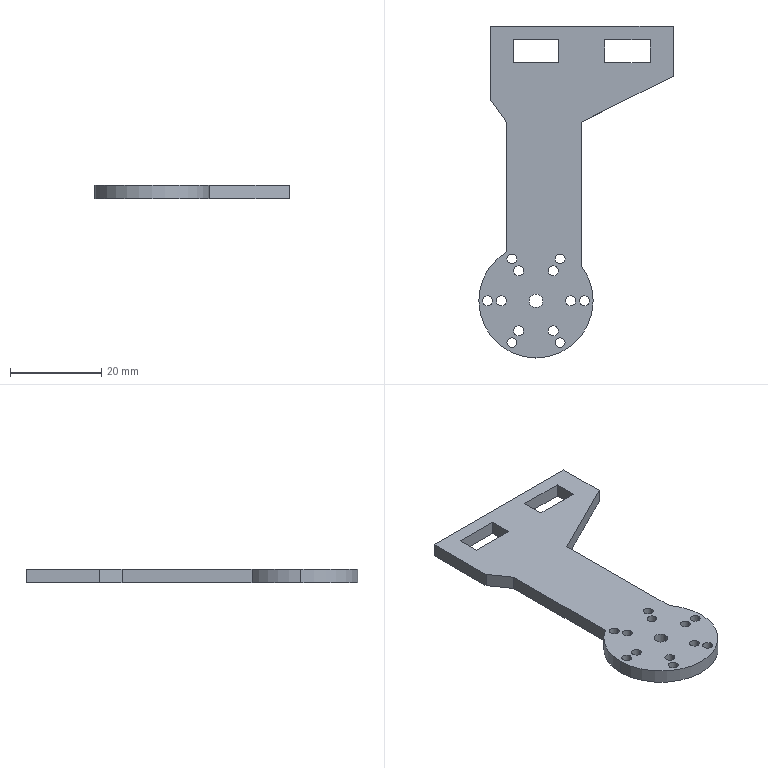Part | SolidWorks | features Extrusion 1 | 1 solid | 46 faces | box 42.5 x 72.6 x 3 mm | volume 4588 mm3 | cylinder 29 | plane 17 | commonest cylinder face diameters 2.15 x24 25 x3 3 x2
STEP:
#1=CARTESIAN_POINT('',(-4.69,-14.849,3.));
#2=VERTEX_POINT('',#1);
#3=CARTESIAN_POINT('',(-2.54,-14.849,3.));
#4=VERTEX_POINT('',#3);
#5=CARTESIAN_POINT('',(-3.615,-14.849,3.));
#6=DIRECTION('',(0.,0.,1.));
#7=DIRECTION('',(1.,0.,0.));
#8=AXIS2_PLACEMENT_3D('',#5,#6,#7);
#9=CIRCLE('',#8,1.075);
#10=EDGE_CURVE('',#2,#4,#9,.T.);
#11=ORIENTED_EDGE('',*,*,#10,.T.);
#12=CARTESIAN_POINT('',(-2.54,-14.849,0.));
#13=VERTEX_POINT('',#12);
#14=CARTESIAN_POINT('',(-2.54,-14.849,3.));
#15=DIRECTION('',(0.,0.,-1.));
#16=VECTOR('',#15,1000.);
#17=LINE('',#14,#16);
#18=EDGE_CURVE('',#4,#13,#17,.T.);
#19=ORIENTED_EDGE('',*,*,#18,.T.);
#20=CARTESIAN_POINT('',(-4.69,-14.849,0.));
#21=VERTEX_POINT('',#20);
#22=CARTESIAN_POINT('',(-3.615,-14.849,0.));
#23=DIRECTION('',(0.,0.,1.));
#24=DIRECTION('',(1.,0.,0.));
#25=AXIS2_PLACEMENT_3D('',#22,#23,#24);
#26=CIRCLE('',#25,1.075);
#27=EDGE_CURVE('',#21,#13,#26,.T.);
#28=ORIENTED_EDGE('',*,*,#27,.F.);
#29=CARTESIAN_POINT('',(-4.69,-14.849,3.));
#30=DIRECTION('',(0.,0.,-1.));
#31=VECTOR('',#30,1000.);
#32=LINE('',#29,#31);
#33=EDGE_CURVE('',#2,#21,#32,.T.);
#34=ORIENTED_EDGE('',*,*,#33,.F.);
#35=EDGE_LOOP('',(#11,#19,#28,#34));
#36=FACE_OUTER_BOUND('',#35,.T.);
#37=CARTESIAN_POINT('',(-3.615,-14.849,3.));
#38=DIRECTION('',(0.,0.,-1.));
#39=DIRECTION('',(-1.,0.,0.));
#40=AXIS2_PLACEMENT_3D('',#37,#38,#39);
#41=CYLINDRICAL_SURFACE('',#40,1.075);
#42=ADVANCED_FACE('',(#36),#41,.F.);
#43=CARTESIAN_POINT('',(-6.19,-17.447,3.));
#44=VERTEX_POINT('',#43);
#45=CARTESIAN_POINT('',(-4.04,-17.447,3.));
#46=VERTEX_POINT('',#45);
#47=CARTESIAN_POINT('',(-5.115,-17.447,3.));
#48=DIRECTION('',(0.,0.,1.));
#49=DIRECTION('',(1.,0.,0.));
#50=AXIS2_PLACEMENT_3D('',#47,#48,#49);
#51=CIRCLE('',#50,1.075);
#52=EDGE_CURVE('',#44,#46,#51,.T.);
#53=ORIENTED_EDGE('',*,*,#52,.T.);
#54=CARTESIAN_POINT('',(-4.04,-17.447,0.));
#55=VERTEX_POINT('',#54);
#56=CARTESIAN_POINT('',(-4.04,-17.447,3.));
#57=DIRECTION('',(0.,0.,-1.));
#58=VECTOR('',#57,1000.);
#59=LINE('',#56,#58);
#60=EDGE_CURVE('',#46,#55,#59,.T.);
#61=ORIENTED_EDGE('',*,*,#60,.T.);
#62=CARTESIAN_POINT('',(-6.19,-17.447,0.));
#63=VERTEX_POINT('',#62);
#64=CARTESIAN_POINT('',(-5.115,-17.447,0.));
#65=DIRECTION('',(0.,0.,1.));
#66=DIRECTION('',(1.,0.,0.));
#67=AXIS2_PLACEMENT_3D('',#64,#65,#66);
#68=CIRCLE('',#67,1.075);
#69=EDGE_CURVE('',#63,#55,#68,.T.);
#70=ORIENTED_EDGE('',*,*,#69,.F.);
#71=CARTESIAN_POINT('',(-6.19,-17.447,3.));
#72=DIRECTION('',(0.,0.,-1.));
#73=VECTOR('',#72,1000.);
#74=LINE('',#71,#73);
#75=EDGE_CURVE('',#44,#63,#74,.T.);
#76=ORIENTED_EDGE('',*,*,#75,.F.);
#77=EDGE_LOOP('',(#53,#61,#70,#76));
#78=FACE_OUTER_BOUND('',#77,.T.);
#79=CARTESIAN_POINT('',(-5.115,-17.447,3.));
#80=DIRECTION('',(0.,0.,-1.));
#81=DIRECTION('',(-1.,0.,0.));
#82=AXIS2_PLACEMENT_3D('',#79,#80,#81);
#83=CYLINDRICAL_SURFACE('',#82,1.075);
#84=ADVANCED_FACE('',(#78),#83,.F.);
#85=CARTESIAN_POINT('',(-15.27,-14.849,3.));
#86=VERTEX_POINT('',#85);
#87=CARTESIAN_POINT('',(-13.12,-14.849,3.));
#88=VERTEX_POINT('',#87);
#89=CARTESIAN_POINT('',(-14.195,-14.849,3.));
#90=DIRECTION('',(0.,0.,1.));
#91=DIRECTION('',(1.,0.,0.));
#92=AXIS2_PLACEMENT_3D('',#89,#90,#91);
#93=CIRCLE('',#92,1.075);
#94=EDGE_CURVE('',#86,#88,#93,.T.);
#95=ORIENTED_EDGE('',*,*,#94,.T.);
#96=CARTESIAN_POINT('',(-13.12,-14.849,0.));
#97=VERTEX_POINT('',#96);
#98=CARTESIAN_POINT('',(-13.12,-14.849,3.));
#99=DIRECTION('',(0.,0.,-1.));
#100=VECTOR('',#99,1000.);
#101=LINE('',#98,#100);
#102=EDGE_CURVE('',#88,#97,#101,.T.);
#103=ORIENTED_EDGE('',*,*,#102,.T.);
#104=CARTESIAN_POINT('',(-15.27,-14.849,0.));
#105=VERTEX_POINT('',#104);
#106=CARTESIAN_POINT('',(-14.195,-14.849,0.));
#107=DIRECTION('',(0.,0.,1.));
#108=DIRECTION('',(1.,0.,0.));
#109=AXIS2_PLACEMENT_3D('',#106,#107,#108);
#110=CIRCLE('',#109,1.075);
#111=EDGE_CURVE('',#105,#97,#110,.T.);
#112=ORIENTED_EDGE('',*,*,#111,.F.);
#113=CARTESIAN_POINT('',(-15.27,-14.849,3.));
#114=DIRECTION('',(0.,0.,-1.));
#115=VECTOR('',#114,1000.);
#116=LINE('',#113,#115);
#117=EDGE_CURVE('',#86,#105,#116,.T.);
#118=ORIENTED_EDGE('',*,*,#117,.F.);
#119=EDGE_LOOP('',(#95,#103,#112,#118));
#120=FACE_OUTER_BOUND('',#119,.T.);
#121=CARTESIAN_POINT('',(-14.195,-14.849,3.));
#122=DIRECTION('',(0.,0.,-1.));
#123=DIRECTION('',(-1.,0.,0.));
#124=AXIS2_PLACEMENT_3D('',#121,#122,#123);
#125=CYLINDRICAL_SURFACE('',#124,1.075);
#126=ADVANCED_FACE('',(#120),#125,.F.);
#127=CARTESIAN_POINT('',(-13.77,-17.447,3.));
#128=VERTEX_POINT('',#127);
#129=CARTESIAN_POINT('',(-11.62,-17.447,3.));
#130=VERTEX_POINT('',#129);
#131=CARTESIAN_POINT('',(-12.695,-17.447,3.));
#132=DIRECTION('',(0.,0.,1.));
#133=DIRECTION('',(1.,0.,0.));
#134=AXIS2_PLACEMENT_3D('',#131,#132,#133);
#135=CIRCLE('',#134,1.075);
#136=EDGE_CURVE('',#128,#130,#135,.T.);
#137=ORIENTED_EDGE('',*,*,#136,.T.);
#138=CARTESIAN_POINT('',(-11.62,-17.447,0.));
#139=VERTEX_POINT('',#138);
#140=CARTESIAN_POINT('',(-11.62,-17.447,3.));
#141=DIRECTION('',(0.,0.,-1.));
#142=VECTOR('',#141,1000.);
#143=LINE('',#140,#142);
#144=EDGE_CURVE('',#130,#139,#143,.T.);
#145=ORIENTED_EDGE('',*,*,#144,.T.);
#146=CARTESIAN_POINT('',(-13.77,-17.447,0.));
#147=VERTEX_POINT('',#146);
#148=CARTESIAN_POINT('',(-12.695,-17.447,0.));
#149=DIRECTION('',(0.,0.,1.));
#150=DIRECTION('',(1.,0.,0.));
#151=AXIS2_PLACEMENT_3D('',#148,#149,#150);
#152=CIRCLE('',#151,1.075);
#153=EDGE_CURVE('',#147,#139,#152,.T.);
#154=ORIENTED_EDGE('',*,*,#153,.F.);
#155=CARTESIAN_POINT('',(-13.77,-17.447,3.));
#156=DIRECTION('',(0.,0.,-1.));
#157=VECTOR('',#156,1000.);
#158=LINE('',#155,#157);
#159=EDGE_CURVE('',#128,#147,#158,.T.);
#160=ORIENTED_EDGE('',*,*,#159,.F.);
#161=EDGE_LOOP('',(#137,#145,#154,#160));
#162=FACE_OUTER_BOUND('',#161,.T.);
#163=CARTESIAN_POINT('',(-12.695,-17.447,3.));
#164=DIRECTION('',(0.,0.,-1.));
#165=DIRECTION('',(-1.,0.,0.));
#166=AXIS2_PLACEMENT_3D('',#163,#164,#165);
#167=CYLINDRICAL_SURFACE('',#166,1.075);
#168=ADVANCED_FACE('',(#162),#167,.F.);
#169=CARTESIAN_POINT('',(-20.56,-24.011,3.));
#170=VERTEX_POINT('',#169);
#171=CARTESIAN_POINT('',(-18.41,-24.011,3.));
#172=VERTEX_POINT('',#171);
#173=CARTESIAN_POINT('',(-19.485,-24.011,3.));
#174=DIRECTION('',(0.,0.,1.));
#175=DIRECTION('',(1.,0.,0.));
#176=AXIS2_PLACEMENT_3D('',#173,#174,#175);
#177=CIRCLE('',#176,1.075);
#178=EDGE_CURVE('',#170,#172,#177,.T.);
#179=ORIENTED_EDGE('',*,*,#178,.T.);
#180=CARTESIAN_POINT('',(-18.41,-24.011,0.));
#181=VERTEX_POINT('',#180);
#182=CARTESIAN_POINT('',(-18.41,-24.011,3.));
#183=DIRECTION('',(0.,0.,-1.));
#184=VECTOR('',#183,1000.);
#185=LINE('',#182,#184);
#186=EDGE_CURVE('',#172,#181,#185,.T.);
#187=ORIENTED_EDGE('',*,*,#186,.T.);
#188=CARTESIAN_POINT('',(-20.56,-24.011,0.));
#189=VERTEX_POINT('',#188);
#190=CARTESIAN_POINT('',(-19.485,-24.011,0.));
#191=DIRECTION('',(0.,0.,1.));
#192=DIRECTION('',(1.,0.,0.));
#193=AXIS2_PLACEMENT_3D('',#190,#191,#192);
#194=CIRCLE('',#193,1.075);
#195=EDGE_CURVE('',#189,#181,#194,.T.);
#196=ORIENTED_EDGE('',*,*,#195,.F.);
#197=CARTESIAN_POINT('',(-20.56,-24.011,3.));
#198=DIRECTION('',(0.,0.,-1.));
#199=VECTOR('',#198,1000.);
#200=LINE('',#197,#199);
#201=EDGE_CURVE('',#170,#189,#200,.T.);
#202=ORIENTED_EDGE('',*,*,#201,.F.);
#203=EDGE_LOOP('',(#179,#187,#196,#202));
#204=FACE_OUTER_BOUND('',#203,.T.);
#205=CARTESIAN_POINT('',(-19.485,-24.011,3.));
#206=DIRECTION('',(0.,0.,-1.));
#207=DIRECTION('',(-1.,0.,0.));
#208=AXIS2_PLACEMENT_3D('',#205,#206,#207);
#209=CYLINDRICAL_SURFACE('',#208,1.075);
#210=ADVANCED_FACE('',(#204),#209,.F.);
#211=CARTESIAN_POINT('',(-17.56,-24.011,3.));
#212=VERTEX_POINT('',#211);
#213=CARTESIAN_POINT('',(-15.41,-24.011,3.));
#214=VERTEX_POINT('',#213);
#215=CARTESIAN_POINT('',(-16.485,-24.011,3.));
#216=DIRECTION('',(0.,0.,1.));
#217=DIRECTION('',(1.,0.,0.));
#218=AXIS2_PLACEMENT_3D('',#215,#216,#217);
#219=CIRCLE('',#218,1.075);
#220=EDGE_CURVE('',#212,#214,#219,.T.);
#221=ORIENTED_EDGE('',*,*,#220,.T.);
#222=CARTESIAN_POINT('',(-15.41,-24.011,0.));
#223=VERTEX_POINT('',#222);
#224=CARTESIAN_POINT('',(-15.41,-24.011,3.));
#225=DIRECTION('',(0.,0.,-1.));
#226=VECTOR('',#225,1000.);
#227=LINE('',#224,#226);
#228=EDGE_CURVE('',#214,#223,#227,.T.);
#229=ORIENTED_EDGE('',*,*,#228,.T.);
#230=CARTESIAN_POINT('',(-17.56,-24.011,0.));
#231=VERTEX_POINT('',#230);
#232=CARTESIAN_POINT('',(-16.485,-24.011,0.));
#233=DIRECTION('',(0.,0.,1.));
#234=DIRECTION('',(1.,0.,0.));
#235=AXIS2_PLACEMENT_3D('',#232,#233,#234);
#236=CIRCLE('',#235,1.075);
#237=EDGE_CURVE('',#231,#223,#236,.T.);
#238=ORIENTED_EDGE('',*,*,#237,.F.);
#239=CARTESIAN_POINT('',(-17.56,-24.011,3.));
#240=DIRECTION('',(0.,0.,-1.));
#241=VECTOR('',#240,1000.);
#242=LINE('',#239,#241);
#243=EDGE_CURVE('',#212,#231,#242,.T.);
#244=ORIENTED_EDGE('',*,*,#243,.F.);
#245=EDGE_LOOP('',(#221,#229,#238,#244));
#246=FACE_OUTER_BOUND('',#245,.T.);
#247=CARTESIAN_POINT('',(-16.485,-24.011,3.));
#248=DIRECTION('',(0.,0.,-1.));
#249=DIRECTION('',(-1.,0.,0.));
#250=AXIS2_PLACEMENT_3D('',#247,#248,#249);
#251=CYLINDRICAL_SURFACE('',#250,1.075);
#252=ADVANCED_FACE('',(#246),#251,.F.);
#253=CARTESIAN_POINT('',(-15.27,-33.174,3.));
#254=VERTEX_POINT('',#253);
#255=CARTESIAN_POINT('',(-13.12,-33.174,3.));
#256=VERTEX_POINT('',#255);
#257=CARTESIAN_POINT('',(-14.195,-33.174,3.));
#258=DIRECTION('',(0.,0.,1.));
#259=DIRECTION('',(1.,0.,0.));
#260=AXIS2_PLACEMENT_3D('',#257,#258,#259);
#261=CIRCLE('',#260,1.075);
#262=EDGE_CURVE('',#254,#256,#261,.T.);
#263=ORIENTED_EDGE('',*,*,#262,.T.);
#264=CARTESIAN_POINT('',(-13.12,-33.174,0.));
#265=VERTEX_POINT('',#264);
#266=CARTESIAN_POINT('',(-13.12,-33.174,3.));
#267=DIRECTION('',(0.,0.,-1.));
#268=VECTOR('',#267,1000.);
#269=LINE('',#266,#268);
#270=EDGE_CURVE('',#256,#265,#269,.T.);
#271=ORIENTED_EDGE('',*,*,#270,.T.);
#272=CARTESIAN_POINT('',(-15.27,-33.174,0.));
#273=VERTEX_POINT('',#272);
#274=CARTESIAN_POINT('',(-14.195,-33.174,0.));
#275=DIRECTION('',(0.,0.,1.));
#276=DIRECTION('',(1.,0.,0.));
#277=AXIS2_PLACEMENT_3D('',#274,#275,#276);
#278=CIRCLE('',#277,1.075);
#279=EDGE_CURVE('',#273,#265,#278,.T.);
#280=ORIENTED_EDGE('',*,*,#279,.F.);
#281=CARTESIAN_POINT('',(-15.27,-33.174,3.));
#282=DIRECTION('',(0.,0.,-1.));
#283=VECTOR('',#282,1000.);
#284=LINE('',#281,#283);
#285=EDGE_CURVE('',#254,#273,#284,.T.);
#286=ORIENTED_EDGE('',*,*,#285,.F.);
#287=EDGE_LOOP('',(#263,#271,#280,#286));
#288=FACE_OUTER_BOUND('',#287,.T.);
#289=CARTESIAN_POINT('',(-14.195,-33.174,3.));
#290=DIRECTION('',(0.,0.,-1.));
#291=DIRECTION('',(-1.,0.,0.));
#292=AXIS2_PLACEMENT_3D('',#289,#290,#291);
#293=CYLINDRICAL_SURFACE('',#292,1.075);
#294=ADVANCED_FACE('',(#288),#293,.F.);
#295=CARTESIAN_POINT('',(-13.77,-30.576,3.));
#296=VERTEX_POINT('',#295);
#297=CARTESIAN_POINT('',(-11.62,-30.576,3.));
#298=VERTEX_POINT('',#297);
#299=CARTESIAN_POINT('',(-12.695,-30.576,3.));
#300=DIRECTION('',(0.,0.,1.));
#301=DIRECTION('',(1.,0.,0.));
#302=AXIS2_PLACEMENT_3D('',#299,#300,#301);
#303=CIRCLE('',#302,1.075);
#304=EDGE_CURVE('',#296,#298,#303,.T.);
#305=ORIENTED_EDGE('',*,*,#304,.T.);
#306=CARTESIAN_POINT('',(-11.62,-30.576,0.));
#307=VERTEX_POINT('',#306);
#308=CARTESIAN_POINT('',(-11.62,-30.576,3.));
#309=DIRECTION('',(0.,0.,-1.));
#310=VECTOR('',#309,1000.);
#311=LINE('',#308,#310);
#312=EDGE_CURVE('',#298,#307,#311,.T.);
#313=ORIENTED_EDGE('',*,*,#312,.T.);
#314=CARTESIAN_POINT('',(-13.77,-30.576,0.));
#315=VERTEX_POINT('',#314);
#316=CARTESIAN_POINT('',(-12.695,-30.576,0.));
#317=DIRECTION('',(0.,0.,1.));
#318=DIRECTION('',(1.,0.,0.));
#319=AXIS2_PLACEMENT_3D('',#316,#317,#318);
#320=CIRCLE('',#319,1.075);
#321=EDGE_CURVE('',#315,#307,#320,.T.);
#322=ORIENTED_EDGE('',*,*,#321,.F.);
#323=CARTESIAN_POINT('',(-13.77,-30.576,3.));
#324=DIRECTION('',(0.,0.,-1.));
#325=VECTOR('',#324,1000.);
#326=LINE('',#323,#325);
#327=EDGE_CURVE('',#296,#315,#326,.T.);
#328=ORIENTED_EDGE('',*,*,#327,.F.);
#329=EDGE_LOOP('',(#305,#313,#322,#328));
#330=FACE_OUTER_BOUND('',#329,.T.);
#331=CARTESIAN_POINT('',(-12.695,-30.576,3.));
#332=DIRECTION('',(0.,0.,-1.));
#333=DIRECTION('',(-1.,0.,0.));
#334=AXIS2_PLACEMENT_3D('',#331,#332,#333);
#335=CYLINDRICAL_SURFACE('',#334,1.075);
#336=ADVANCED_FACE('',(#330),#335,.F.);
#337=CARTESIAN_POINT('',(-4.69,-33.174,3.));
#338=VERTEX_POINT('',#337);
#339=CARTESIAN_POINT('',(-2.54,-33.174,3.));
#340=VERTEX_POINT('',#339);
#341=CARTESIAN_POINT('',(-3.615,-33.174,3.));
#342=DIRECTION('',(0.,0.,1.));
#343=DIRECTION('',(1.,0.,0.));
#344=AXIS2_PLACEMENT_3D('',#341,#342,#343);
#345=CIRCLE('',#344,1.075);
#346=EDGE_CURVE('',#338,#340,#345,.T.);
#347=ORIENTED_EDGE('',*,*,#346,.T.);
#348=CARTESIAN_POINT('',(-2.54,-33.174,0.));
#349=VERTEX_POINT('',#348);
#350=CARTESIAN_POINT('',(-2.54,-33.174,3.));
#351=DIRECTION('',(0.,0.,-1.));
#352=VECTOR('',#351,1000.);
#353=LINE('',#350,#352);
#354=EDGE_CURVE('',#340,#349,#353,.T.);
#355=ORIENTED_EDGE('',*,*,#354,.T.);
#356=CARTESIAN_POINT('',(-4.69,-33.174,0.));
#357=VERTEX_POINT('',#356);
#358=CARTESIAN_POINT('',(-3.615,-33.174,0.));
#359=DIRECTION('',(0.,0.,1.));
#360=DIRECTION('',(1.,0.,0.));
#361=AXIS2_PLACEMENT_3D('',#358,#359,#360);
#362=CIRCLE('',#361,1.075);
#363=EDGE_CURVE('',#357,#349,#362,.T.);
#364=ORIENTED_EDGE('',*,*,#363,.F.);
#365=CARTESIAN_POINT('',(-4.69,-33.174,3.));
#366=DIRECTION('',(0.,0.,-1.));
#367=VECTOR('',#366,1000.);
#368=LINE('',#365,#367);
#369=EDGE_CURVE('',#338,#357,#368,.T.);
#370=ORIENTED_EDGE('',*,*,#369,.F.);
#371=EDGE_LOOP('',(#347,#355,#364,#370));
#372=FACE_OUTER_BOUND('',#371,.T.);
#373=CARTESIAN_POINT('',(-3.615,-33.174,3.));
#374=DIRECTION('',(0.,0.,-1.));
#375=DIRECTION('',(-1.,0.,0.));
#376=AXIS2_PLACEMENT_3D('',#373,#374,#375);
#377=CYLINDRICAL_SURFACE('',#376,1.075);
#378=ADVANCED_FACE('',(#372),#377,.F.);
#379=CARTESIAN_POINT('',(-6.19,-30.576,3.));
#380=VERTEX_POINT('',#379);
#381=CARTESIAN_POINT('',(-4.04,-30.576,3.));
#382=VERTEX_POINT('',#381);
#383=CARTESIAN_POINT('',(-5.115,-30.576,3.));
#384=DIRECTION('',(0.,0.,1.));
#385=DIRECTION('',(1.,0.,0.));
#386=AXIS2_PLACEMENT_3D('',#383,#384,#385);
#387=CIRCLE('',#386,1.075);
#388=EDGE_CURVE('',#380,#382,#387,.T.);
#389=ORIENTED_EDGE('',*,*,#388,.T.);
#390=CARTESIAN_POINT('',(-4.04,-30.576,0.));
#391=VERTEX_POINT('',#390);
#392=CARTESIAN_POINT('',(-4.04,-30.576,3.));
#393=DIRECTION('',(0.,0.,-1.));
#394=VECTOR('',#393,1000.);
#395=LINE('',#392,#394);
#396=EDGE_CURVE('',#382,#391,#395,.T.);
#397=ORIENTED_EDGE('',*,*,#396,.T.);
#398=CARTESIAN_POINT('',(-6.19,-30.576,0.));
#399=VERTEX_POINT('',#398);
#400=CARTESIAN_POINT('',(-5.115,-30.576,0.));
#401=DIRECTION('',(0.,0.,1.));
#402=DIRECTION('',(1.,0.,0.));
#403=AXIS2_PLACEMENT_3D('',#400,#401,#402);
#404=CIRCLE('',#403,1.075);
#405=EDGE_CURVE('',#399,#391,#404,.T.);
#406=ORIENTED_EDGE('',*,*,#405,.F.);
#407=CARTESIAN_POINT('',(-6.19,-30.576,3.));
#408=DIRECTION('',(0.,0.,-1.));
#409=VECTOR('',#408,1000.);
#410=LINE('',#407,#409);
#411=EDGE_CURVE('',#380,#399,#410,.T.);
#412=ORIENTED_EDGE('',*,*,#411,.F.);
#413=EDGE_LOOP('',(#389,#397,#406,#412));
#414=FACE_OUTER_BOUND('',#413,.T.);
#415=CARTESIAN_POINT('',(-5.115,-30.576,3.));
#416=DIRECTION('',(0.,0.,-1.));
#417=DIRECTION('',(-1.,0.,0.));
#418=AXIS2_PLACEMENT_3D('',#415,#416,#417);
#419=CYLINDRICAL_SURFACE('',#418,1.075);
#420=ADVANCED_FACE('',(#414),#419,.F.);
#421=CARTESIAN_POINT('',(0.6,-24.011,3.));
#422=VERTEX_POINT('',#421);
#423=CARTESIAN_POINT('',(2.75,-24.011,3.));
#424=VERTEX_POINT('',#423);
#425=CARTESIAN_POINT('',(1.675,-24.011,3.));
#426=DIRECTION('',(0.,0.,1.));
#427=DIRECTION('',(1.,0.,0.));
#428=AXIS2_PLACEMENT_3D('',#425,#426,#427);
#429=CIRCLE('',#428,1.075);
#430=EDGE_CURVE('',#422,#424,#429,.T.);
#431=ORIENTED_EDGE('',*,*,#430,.T.);
#432=CARTESIAN_POINT('',(2.75,-24.011,0.));
#433=VERTEX_POINT('',#432);
#434=CARTESIAN_POINT('',(2.75,-24.011,3.));
#435=DIRECTION('',(0.,0.,-1.));
#436=VECTOR('',#435,1000.);
#437=LINE('',#434,#436);
#438=EDGE_CURVE('',#424,#433,#437,.T.);
#439=ORIENTED_EDGE('',*,*,#438,.T.);
#440=CARTESIAN_POINT('',(0.6,-24.011,0.));
#441=VERTEX_POINT('',#440);
#442=CARTESIAN_POINT('',(1.675,-24.011,0.));
#443=DIRECTION('',(0.,0.,1.));
#444=DIRECTION('',(1.,0.,0.));
#445=AXIS2_PLACEMENT_3D('',#442,#443,#444);
#446=CIRCLE('',#445,1.075);
#447=EDGE_CURVE('',#441,#433,#446,.T.);
#448=ORIENTED_EDGE('',*,*,#447,.F.);
#449=CARTESIAN_POINT('',(0.6,-24.011,3.));
#450=DIRECTION('',(0.,0.,-1.));
#451=VECTOR('',#450,1000.);
#452=LINE('',#449,#451);
#453=EDGE_CURVE('',#422,#441,#452,.T.);
#454=ORIENTED_EDGE('',*,*,#453,.F.);
#455=EDGE_LOOP('',(#431,#439,#448,#454));
#456=FACE_OUTER_BOUND('',#455,.T.);
#457=CARTESIAN_POINT('',(1.675,-24.011,3.));
#458=DIRECTION('',(0.,0.,-1.));
#459=DIRECTION('',(-1.,0.,0.));
#460=AXIS2_PLACEMENT_3D('',#457,#458,#459);
#461=CYLINDRICAL_SURFACE('',#460,1.075);
#462=ADVANCED_FACE('',(#456),#461,.F.);
#463=CARTESIAN_POINT('',(-10.405,-24.011,3.));
#464=VERTEX_POINT('',#463);
#465=CARTESIAN_POINT('',(-7.405,-24.011,3.));
#466=VERTEX_POINT('',#465);
#467=CARTESIAN_POINT('',(-8.905,-24.011,3.));
#468=DIRECTION('',(0.,0.,1.));
#469=DIRECTION('',(1.,0.,0.));
#470=AXIS2_PLACEMENT_3D('',#467,#468,#469);
#471=CIRCLE('',#470,1.5);
#472=EDGE_CURVE('',#464,#466,#471,.T.);
#473=ORIENTED_EDGE('',*,*,#472,.T.);
#474=CARTESIAN_POINT('',(-7.405,-24.011,0.));
#475=VERTEX_POINT('',#474);
#476=CARTESIAN_POINT('',(-7.405,-24.011,3.));
#477=DIRECTION('',(0.,0.,-1.));
#478=VECTOR('',#477,1000.);
#479=LINE('',#476,#478);
#480=EDGE_CURVE('',#466,#475,#479,.T.);
#481=ORIENTED_EDGE('',*,*,#480,.T.);
#482=CARTESIAN_POINT('',(-10.405,-24.011,0.));
#483=VERTEX_POINT('',#482);
#484=CARTESIAN_POINT('',(-8.905,-24.011,0.));
#485=DIRECTION('',(0.,0.,1.));
#486=DIRECTION('',(1.,0.,0.));
#487=AXIS2_PLACEMENT_3D('',#484,#485,#486);
#488=CIRCLE('',#487,1.5);
#489=EDGE_CURVE('',#483,#475,#488,.T.);
#490=ORIENTED_EDGE('',*,*,#489,.F.);
#491=CARTESIAN_POINT('',(-10.405,-24.011,3.));
#492=DIRECTION('',(0.,0.,-1.));
#493=VECTOR('',#492,1000.);
#494=LINE('',#491,#493);
#495=EDGE_CURVE('',#464,#483,#494,.T.);
#496=ORIENTED_EDGE('',*,*,#495,.F.);
#497=EDGE_LOOP('',(#473,#481,#490,#496));
#498=FACE_OUTER_BOUND('',#497,.T.);
#499=CARTESIAN_POINT('',(-8.905,-24.011,3.));
#500=DIRECTION('',(0.,0.,-1.));
#501=DIRECTION('',(-1.,0.,0.));
#502=AXIS2_PLACEMENT_3D('',#499,#500,#501);
#503=CYLINDRICAL_SURFACE('',#502,1.5);
#504=ADVANCED_FACE('',(#498),#503,.F.);
#505=CARTESIAN_POINT('',(-2.4,-24.011,3.));
#506=VERTEX_POINT('',#505);
#507=CARTESIAN_POINT('',(-0.25,-24.011,3.));
#508=VERTEX_POINT('',#507);
#509=CARTESIAN_POINT('',(-1.325,-24.011,3.));
#510=DIRECTION('',(0.,0.,1.));
#511=DIRECTION('',(1.,0.,0.));
#512=AXIS2_PLACEMENT_3D('',#509,#510,#511);
#513=CIRCLE('',#512,1.075);
#514=EDGE_CURVE('',#506,#508,#513,.T.);
#515=ORIENTED_EDGE('',*,*,#514,.T.);
#516=CARTESIAN_POINT('',(-0.25,-24.011,0.));
#517=VERTEX_POINT('',#516);
#518=CARTESIAN_POINT('',(-0.25,-24.011,3.));
#519=DIRECTION('',(0.,0.,-1.));
#520=VECTOR('',#519,1000.);
#521=LINE('',#518,#520);
#522=EDGE_CURVE('',#508,#517,#521,.T.);
#523=ORIENTED_EDGE('',*,*,#522,.T.);
#524=CARTESIAN_POINT('',(-2.4,-24.011,0.));
#525=VERTEX_POINT('',#524);
#526=CARTESIAN_POINT('',(-1.325,-24.011,0.));
#527=DIRECTION('',(0.,0.,1.));
#528=DIRECTION('',(1.,0.,0.));
#529=AXIS2_PLACEMENT_3D('',#526,#527,#528);
#530=CIRCLE('',#529,1.075);
#531=EDGE_CURVE('',#525,#517,#530,.T.);
#532=ORIENTED_EDGE('',*,*,#531,.F.);
#533=CARTESIAN_POINT('',(-2.4,-24.011,3.));
#534=DIRECTION('',(0.,0.,-1.));
#535=VECTOR('',#534,1000.);
#536=LINE('',#533,#535);
#537=EDGE_CURVE('',#506,#525,#536,.T.);
#538=ORIENTED_EDGE('',*,*,#537,.F.);
#539=EDGE_LOOP('',(#515,#523,#532,#538));
#540=FACE_OUTER_BOUND('',#539,.T.);
#541=CARTESIAN_POINT('',(-1.325,-24.011,3.));
#542=DIRECTION('',(0.,0.,-1.));
#543=DIRECTION('',(-1.,0.,0.));
#544=AXIS2_PLACEMENT_3D('',#541,#542,#543);
#545=CYLINDRICAL_SURFACE('',#544,1.075);
#546=ADVANCED_FACE('',(#540),#545,.F.);
#547=CARTESIAN_POINT('',(3.595,-24.011,3.));
#548=VERTEX_POINT('',#547);
#549=CARTESIAN_POINT('',(1.095,-16.511,3.));
#550=VERTEX_POINT('',#549);
#551=CARTESIAN_POINT('',(-8.905,-24.011,3.));
#552=DIRECTION('',(0.,0.,1.));
#553=DIRECTION('',(1.,0.,0.));
#554=AXIS2_PLACEMENT_3D('',#551,#552,#553);
#555=CIRCLE('',#554,12.5);
#556=EDGE_CURVE('',#548,#550,#555,.T.);
#557=ORIENTED_EDGE('',*,*,#556,.F.);
#558=CARTESIAN_POINT('',(3.595,-24.011,0.));
#559=VERTEX_POINT('',#558);
#560=CARTESIAN_POINT('',(3.595,-24.011,3.));
#561=DIRECTION('',(0.,0.,-1.));
#562=VECTOR('',#561,1000.);
#563=LINE('',#560,#562);
#564=EDGE_CURVE('',#548,#559,#563,.T.);
#565=ORIENTED_EDGE('',*,*,#564,.T.);
#566=CARTESIAN_POINT('',(1.095,-16.511,0.));
#567=VERTEX_POINT('',#566);
#568=CARTESIAN_POINT('',(-8.905,-24.011,0.));
#569=DIRECTION('',(0.,0.,1.));
#570=DIRECTION('',(1.,0.,0.));
#571=AXIS2_PLACEMENT_3D('',#568,#569,#570);
#572=CIRCLE('',#571,12.5);
#573=EDGE_CURVE('',#559,#567,#572,.T.);
#574=ORIENTED_EDGE('',*,*,#573,.T.);
#575=CARTESIAN_POINT('',(1.095,-16.511,3.));
#576=DIRECTION('',(0.,0.,-1.));
#577=VECTOR('',#576,1000.);
#578=LINE('',#575,#577);
#579=EDGE_CURVE('',#550,#567,#578,.T.);
#580=ORIENTED_EDGE('',*,*,#579,.F.);
#581=EDGE_LOOP('',(#557,#565,#574,#580));
#582=FACE_OUTER_BOUND('',#581,.T.);
#583=CARTESIAN_POINT('',(-8.905,-24.011,3.));
#584=DIRECTION('',(0.,0.,-1.));
#585=DIRECTION('',(-1.,0.,0.));
#586=AXIS2_PLACEMENT_3D('',#583,#584,#585);
#587=CYLINDRICAL_SURFACE('',#586,12.5);
#588=ADVANCED_FACE('',(#582),#587,.T.);
#589=ORIENTED_EDGE('',*,*,#564,.F.);
#590=CARTESIAN_POINT('',(-21.405,-24.011,3.));
#591=VERTEX_POINT('',#590);
#592=CARTESIAN_POINT('',(-8.905,-24.011,3.));
#593=DIRECTION('',(0.,0.,1.));
#594=DIRECTION('',(1.,0.,0.));
#595=AXIS2_PLACEMENT_3D('',#592,#593,#594);
#596=CIRCLE('',#595,12.5);
#597=EDGE_CURVE('',#591,#548,#596,.T.);
#598=ORIENTED_EDGE('',*,*,#597,.F.);
#599=CARTESIAN_POINT('',(-21.405,-24.011,0.));
#600=VERTEX_POINT('',#599);
#601=CARTESIAN_POINT('',(-21.405,-24.011,3.));
#602=DIRECTION('',(0.,0.,-1.));
#603=VECTOR('',#602,1000.);
#604=LINE('',#601,#603);
#605=EDGE_CURVE('',#591,#600,#604,.T.);
#606=ORIENTED_EDGE('',*,*,#605,.T.);
#607=CARTESIAN_POINT('',(-8.905,-24.011,0.));
#608=DIRECTION('',(0.,0.,1.));
#609=DIRECTION('',(1.,0.,0.));
#610=AXIS2_PLACEMENT_3D('',#607,#608,#609);
#611=CIRCLE('',#610,12.5);
#612=EDGE_CURVE('',#600,#559,#611,.T.);
#613=ORIENTED_EDGE('',*,*,#612,.T.);
#614=EDGE_LOOP('',(#589,#598,#606,#613));
#615=FACE_OUTER_BOUND('',#614,.T.);
#616=CARTESIAN_POINT('',(-8.905,-24.011,3.));
#617=DIRECTION('',(0.,0.,-1.));
#618=DIRECTION('',(-1.,0.,0.));
#619=AXIS2_PLACEMENT_3D('',#616,#617,#618);
#620=CYLINDRICAL_SURFACE('',#619,12.5);
#621=ADVANCED_FACE('',(#615),#620,.T.);
#622=ORIENTED_EDGE('',*,*,#52,.F.);
#623=CARTESIAN_POINT('',(-5.115,-17.447,3.));
#624=DIRECTION('',(0.,0.,1.));
#625=DIRECTION('',(1.,0.,0.));
#626=AXIS2_PLACEMENT_3D('',#623,#624,#625);
#627=CIRCLE('',#626,1.075);
#628=EDGE_CURVE('',#46,#44,#627,.T.);
#629=ORIENTED_EDGE('',*,*,#628,.F.);
#630=EDGE_LOOP('',(#622,#629));
#631=FACE_BOUND('',#630,.T.);
#632=ORIENTED_EDGE('',*,*,#136,.F.);
#633=CARTESIAN_POINT('',(-12.695,-17.447,3.));
#634=DIRECTION('',(0.,0.,1.));
#635=DIRECTION('',(1.,0.,0.));
#636=AXIS2_PLACEMENT_3D('',#633,#634,#635);
#637=CIRCLE('',#636,1.075);
#638=EDGE_CURVE('',#130,#128,#637,.T.);
#639=ORIENTED_EDGE('',*,*,#638,.F.);
#640=EDGE_LOOP('',(#632,#639));
#641=FACE_BOUND('',#640,.T.);
#642=ORIENTED_EDGE('',*,*,#220,.F.);
#643=CARTESIAN_POINT('',(-16.485,-24.011,3.));
#644=DIRECTION('',(0.,0.,1.));
#645=DIRECTION('',(1.,0.,0.));
#646=AXIS2_PLACEMENT_3D('',#643,#644,#645);
#647=CIRCLE('',#646,1.075);
#648=EDGE_CURVE('',#214,#212,#647,.T.);
#649=ORIENTED_EDGE('',*,*,#648,.F.);
#650=EDGE_LOOP('',(#642,#649));
#651=FACE_BOUND('',#650,.T.);
#652=ORIENTED_EDGE('',*,*,#304,.F.);
#653=CARTESIAN_POINT('',(-12.695,-30.576,3.));
#654=DIRECTION('',(0.,0.,1.));
#655=DIRECTION('',(1.,0.,0.));
#656=AXIS2_PLACEMENT_3D('',#653,#654,#655);
#657=CIRCLE('',#656,1.075);
#658=EDGE_CURVE('',#298,#296,#657,.T.);
#659=ORIENTED_EDGE('',*,*,#658,.F.);
#660=EDGE_LOOP('',(#652,#659));
#661=FACE_BOUND('',#660,.T.);
#662=CARTESIAN_POINT('',(-13.905,28.089,3.));
#663=VERTEX_POINT('',#662);
#664=CARTESIAN_POINT('',(-3.905,28.089,3.));
#665=VERTEX_POINT('',#664);
#666=CARTESIAN_POINT('',(-13.905,28.089,3.));
#667=DIRECTION('',(1.,0.,0.));
#668=VECTOR('',#667,1000.);
#669=LINE('',#666,#668);
#670=EDGE_CURVE('',#663,#665,#669,.T.);
#671=ORIENTED_EDGE('',*,*,#670,.F.);
#672=CARTESIAN_POINT('',(-13.905,33.089,3.));
#673=VERTEX_POINT('',#672);
#674=CARTESIAN_POINT('',(-13.905,28.089,3.));
#675=DIRECTION('',(0.,-1.,0.));
#676=VECTOR('',#675,1000.);
#677=LINE('',#674,#676);
#678=EDGE_CURVE('',#673,#663,#677,.T.);
#679=ORIENTED_EDGE('',*,*,#678,.F.);
#680=CARTESIAN_POINT('',(-3.905,33.089,3.));
#681=VERTEX_POINT('',#680);
#682=CARTESIAN_POINT('',(-13.905,33.089,3.));
#683=DIRECTION('',(-1.,0.,0.));
#684=VECTOR('',#683,1000.);
#685=LINE('',#682,#684);
#686=EDGE_CURVE('',#681,#673,#685,.T.);
#687=ORIENTED_EDGE('',*,*,#686,.F.);
#688=CARTESIAN_POINT('',(-3.905,28.089,3.));
#689=DIRECTION('',(0.,1.,0.));
#690=VECTOR('',#689,1000.);
#691=LINE('',#688,#690);
#692=EDGE_CURVE('',#665,#681,#691,.T.);
#693=ORIENTED_EDGE('',*,*,#692,.F.);
#694=EDGE_LOOP('',(#671,#679,#687,#693));
#695=FACE_BOUND('',#694,.T.);
#696=ORIENTED_EDGE('',*,*,#388,.F.);
#697=CARTESIAN_POINT('',(-5.115,-30.576,3.));
#698=DIRECTION('',(0.,0.,1.));
#699=DIRECTION('',(1.,0.,0.));
#700=AXIS2_PLACEMENT_3D('',#697,#698,#699);
#701=CIRCLE('',#700,1.075);
#702=EDGE_CURVE('',#382,#380,#701,.T.);
#703=ORIENTED_EDGE('',*,*,#702,.F.);
#704=EDGE_LOOP('',(#696,#703));
#705=FACE_BOUND('',#704,.T.);
#706=ORIENTED_EDGE('',*,*,#472,.F.);
#707=CARTESIAN_POINT('',(-8.905,-24.011,3.));
#708=DIRECTION('',(0.,0.,1.));
#709=DIRECTION('',(1.,0.,0.));
#710=AXIS2_PLACEMENT_3D('',#707,#708,#709);
#711=CIRCLE('',#710,1.5);
#712=EDGE_CURVE('',#466,#464,#711,.T.);
#713=ORIENTED_EDGE('',*,*,#712,.F.);
#714=EDGE_LOOP('',(#706,#713));
#715=FACE_BOUND('',#714,.T.);
#716=CARTESIAN_POINT('',(6.095,28.089,3.));
#717=VERTEX_POINT('',#716);
#718=CARTESIAN_POINT('',(16.095,28.089,3.));
#719=VERTEX_POINT('',#718);
#720=CARTESIAN_POINT('',(6.095,28.089,3.));
#721=DIRECTION('',(1.,0.,0.));
#722=VECTOR('',#721,1000.);
#723=LINE('',#720,#722);
#724=EDGE_CURVE('',#717,#719,#723,.T.);
#725=ORIENTED_EDGE('',*,*,#724,.F.);
#726=CARTESIAN_POINT('',(6.095,33.089,3.));
#727=VERTEX_POINT('',#726);
#728=CARTESIAN_POINT('',(6.095,28.089,3.));
#729=DIRECTION('',(0.,-1.,0.));
#730=VECTOR('',#729,1000.);
#731=LINE('',#728,#730);
#732=EDGE_CURVE('',#727,#717,#731,.T.);
#733=ORIENTED_EDGE('',*,*,#732,.F.);
#734=CARTESIAN_POINT('',(16.095,33.089,3.));
#735=VERTEX_POINT('',#734);
#736=CARTESIAN_POINT('',(6.095,33.089,3.));
#737=DIRECTION('',(-1.,0.,0.));
#738=VECTOR('',#737,1000.);
#739=LINE('',#736,#738);
#740=EDGE_CURVE('',#735,#727,#739,.T.);
#741=ORIENTED_EDGE('',*,*,#740,.F.);
#742=CARTESIAN_POINT('',(16.095,28.089,3.));
#743=DIRECTION('',(0.,1.,0.));
#744=VECTOR('',#743,1000.);
#745=LINE('',#742,#744);
#746=EDGE_CURVE('',#719,#735,#745,.T.);
#747=ORIENTED_EDGE('',*,*,#746,.F.);
#748=EDGE_LOOP('',(#725,#733,#741,#747));
#749=FACE_BOUND('',#748,.T.);
#750=CARTESIAN_POINT('',(-15.405,-13.334,3.));
#751=VERTEX_POINT('',#750);
#752=CARTESIAN_POINT('',(-8.905,-24.011,3.));
#753=DIRECTION('',(0.,0.,1.));
#754=DIRECTION('',(1.,0.,0.));
#755=AXIS2_PLACEMENT_3D('',#752,#753,#754);
#756=CIRCLE('',#755,12.5);
#757=EDGE_CURVE('',#751,#591,#756,.T.);
#758=ORIENTED_EDGE('',*,*,#757,.T.);
#759=ORIENTED_EDGE('',*,*,#597,.T.);
#760=ORIENTED_EDGE('',*,*,#556,.T.);
#761=CARTESIAN_POINT('',(1.095,15.089,3.));
#762=VERTEX_POINT('',#761);
#763=CARTESIAN_POINT('',(1.095,15.089,3.));
#764=DIRECTION('',(0.,1.,0.));
#765=VECTOR('',#764,1000.);
#766=LINE('',#763,#765);
#767=EDGE_CURVE('',#550,#762,#766,.T.);
#768=ORIENTED_EDGE('',*,*,#767,.T.);
#769=CARTESIAN_POINT('',(21.095,25.089,3.));
#770=VERTEX_POINT('',#769);
#771=CARTESIAN_POINT('',(21.095,25.089,3.));
#772=DIRECTION('',(0.8944,0.4472,0.));
#773=VECTOR('',#772,1000.);
#774=LINE('',#771,#773);
#775=EDGE_CURVE('',#762,#770,#774,.T.);
#776=ORIENTED_EDGE('',*,*,#775,.T.);
#777=CARTESIAN_POINT('',(21.095,36.089,3.));
#778=VERTEX_POINT('',#777);
#779=CARTESIAN_POINT('',(21.095,36.089,3.));
#780=DIRECTION('',(0.,1.,0.));
#781=VECTOR('',#780,1000.);
#782=LINE('',#779,#781);
#783=EDGE_CURVE('',#770,#778,#782,.T.);
#784=ORIENTED_EDGE('',*,*,#783,.T.);
#785=CARTESIAN_POINT('',(-18.905,36.089,3.));
#786=VERTEX_POINT('',#785);
#787=CARTESIAN_POINT('',(-18.905,36.089,3.));
#788=DIRECTION('',(-1.,0.,0.));
#789=VECTOR('',#788,1000.);
#790=LINE('',#787,#789);
#791=EDGE_CURVE('',#778,#786,#790,.T.);
#792=ORIENTED_EDGE('',*,*,#791,.T.);
#793=CARTESIAN_POINT('',(-18.905,20.089,3.));
#794=VERTEX_POINT('',#793);
#795=CARTESIAN_POINT('',(-18.905,20.089,3.));
#796=DIRECTION('',(0.,-1.,0.));
#797=VECTOR('',#796,1000.);
#798=LINE('',#795,#797);
#799=EDGE_CURVE('',#786,#794,#798,.T.);
#800=ORIENTED_EDGE('',*,*,#799,.T.);
#801=CARTESIAN_POINT('',(-15.405,15.09,3.));
#802=VERTEX_POINT('',#801);
#803=CARTESIAN_POINT('',(-15.405,15.09,3.));
#804=DIRECTION('',(0.5736,-0.8192,0.));
#805=VECTOR('',#804,1000.);
#806=LINE('',#803,#805);
#807=EDGE_CURVE('',#794,#802,#806,.T.);
#808=ORIENTED_EDGE('',*,*,#807,.T.);
#809=CARTESIAN_POINT('',(-15.405,-13.334,3.));
#810=DIRECTION('',(0.,-1.,0.));
#811=VECTOR('',#810,1000.);
#812=LINE('',#809,#811);
#813=EDGE_CURVE('',#802,#751,#812,.T.);
#814=ORIENTED_EDGE('',*,*,#813,.T.);
#815=EDGE_LOOP('',(#758,#759,#760,#768,#776,#784,#792,#800,#808,#814));
#816=FACE_OUTER_BOUND('',#815,.T.);
#817=ORIENTED_EDGE('',*,*,#514,.F.);
#818=CARTESIAN_POINT('',(-1.325,-24.011,3.));
#819=DIRECTION('',(0.,0.,1.));
#820=DIRECTION('',(1.,0.,0.));
#821=AXIS2_PLACEMENT_3D('',#818,#819,#820);
#822=CIRCLE('',#821,1.075);
#823=EDGE_CURVE('',#508,#506,#822,.T.);
#824=ORIENTED_EDGE('',*,*,#823,.F.);
#825=EDGE_LOOP('',(#817,#824));
#826=FACE_BOUND('',#825,.T.);
#827=ORIENTED_EDGE('',*,*,#430,.F.);
#828=CARTESIAN_POINT('',(1.675,-24.011,3.));
#829=DIRECTION('',(0.,0.,1.));
#830=DIRECTION('',(1.,0.,0.));
#831=AXIS2_PLACEMENT_3D('',#828,#829,#830);
#832=CIRCLE('',#831,1.075);
#833=EDGE_CURVE('',#424,#422,#832,.T.);
#834=ORIENTED_EDGE('',*,*,#833,.F.);
#835=EDGE_LOOP('',(#827,#834));
#836=FACE_BOUND('',#835,.T.);
#837=ORIENTED_EDGE('',*,*,#346,.F.);
#838=CARTESIAN_POINT('',(-3.615,-33.174,3.));
#839=DIRECTION('',(0.,0.,1.));
#840=DIRECTION('',(1.,0.,0.));
#841=AXIS2_PLACEMENT_3D('',#838,#839,#840);
#842=CIRCLE('',#841,1.075);
#843=EDGE_CURVE('',#340,#338,#842,.T.);
#844=ORIENTED_EDGE('',*,*,#843,.F.);
#845=EDGE_LOOP('',(#837,#844));
#846=FACE_BOUND('',#845,.T.);
#847=ORIENTED_EDGE('',*,*,#262,.F.);
#848=CARTESIAN_POINT('',(-14.195,-33.174,3.));
#849=DIRECTION('',(0.,0.,1.));
#850=DIRECTION('',(1.,0.,0.));
#851=AXIS2_PLACEMENT_3D('',#848,#849,#850);
#852=CIRCLE('',#851,1.075);
#853=EDGE_CURVE('',#256,#254,#852,.T.);
#854=ORIENTED_EDGE('',*,*,#853,.F.);
#855=EDGE_LOOP('',(#847,#854));
#856=FACE_BOUND('',#855,.T.);
#857=ORIENTED_EDGE('',*,*,#178,.F.);
#858=CARTESIAN_POINT('',(-19.485,-24.011,3.));
#859=DIRECTION('',(0.,0.,1.));
#860=DIRECTION('',(1.,0.,0.));
#861=AXIS2_PLACEMENT_3D('',#858,#859,#860);
#862=CIRCLE('',#861,1.075);
#863=EDGE_CURVE('',#172,#170,#862,.T.);
#864=ORIENTED_EDGE('',*,*,#863,.F.);
#865=EDGE_LOOP('',(#857,#864));
#866=FACE_BOUND('',#865,.T.);
#867=ORIENTED_EDGE('',*,*,#94,.F.);
#868=CARTESIAN_POINT('',(-14.195,-14.849,3.));
#869=DIRECTION('',(0.,0.,1.));
#870=DIRECTION('',(1.,0.,0.));
#871=AXIS2_PLACEMENT_3D('',#868,#869,#870);
#872=CIRCLE('',#871,1.075);
#873=EDGE_CURVE('',#88,#86,#872,.T.);
#874=ORIENTED_EDGE('',*,*,#873,.F.);
#875=EDGE_LOOP('',(#867,#874));
#876=FACE_BOUND('',#875,.T.);
#877=ORIENTED_EDGE('',*,*,#10,.F.);
#878=CARTESIAN_POINT('',(-3.615,-14.849,3.));
#879=DIRECTION('',(0.,0.,1.));
#880=DIRECTION('',(1.,0.,0.));
#881=AXIS2_PLACEMENT_3D('',#878,#879,#880);
#882=CIRCLE('',#881,1.075);
#883=EDGE_CURVE('',#4,#2,#882,.T.);
#884=ORIENTED_EDGE('',*,*,#883,.F.);
#885=EDGE_LOOP('',(#877,#884));
#886=FACE_BOUND('',#885,.T.);
#887=CARTESIAN_POINT('',(-8.905,-24.011,3.));
#888=DIRECTION('',(0.,0.,1.));
#889=DIRECTION('',(1.,0.,0.));
#890=AXIS2_PLACEMENT_3D('',#887,#888,#889);
#891=PLANE('',#890);
#892=ADVANCED_FACE('',(#631,#641,#651,#661,#695,#705,#715,#749,#816,#826,#836,#846,#856,#866,#876,#886),#891,.T.);
#893=ORIENTED_EDGE('',*,*,#405,.T.);
#894=CARTESIAN_POINT('',(-5.115,-30.576,0.));
#895=DIRECTION('',(0.,0.,1.));
#896=DIRECTION('',(1.,0.,0.));
#897=AXIS2_PLACEMENT_3D('',#894,#895,#896);
#898=CIRCLE('',#897,1.075);
#899=EDGE_CURVE('',#391,#399,#898,.T.);
#900=ORIENTED_EDGE('',*,*,#899,.T.);
#901=EDGE_LOOP('',(#893,#900));
#902=FACE_BOUND('',#901,.T.);
#903=ORIENTED_EDGE('',*,*,#447,.T.);
#904=CARTESIAN_POINT('',(1.675,-24.011,0.));
#905=DIRECTION('',(0.,0.,1.));
#906=DIRECTION('',(1.,0.,0.));
#907=AXIS2_PLACEMENT_3D('',#904,#905,#906);
#908=CIRCLE('',#907,1.075);
#909=EDGE_CURVE('',#433,#441,#908,.T.);
#910=ORIENTED_EDGE('',*,*,#909,.T.);
#911=EDGE_LOOP('',(#903,#910));
#912=FACE_BOUND('',#911,.T.);
#913=ORIENTED_EDGE('',*,*,#489,.T.);
#914=CARTESIAN_POINT('',(-8.905,-24.011,0.));
#915=DIRECTION('',(0.,0.,1.));
#916=DIRECTION('',(1.,0.,0.));
#917=AXIS2_PLACEMENT_3D('',#914,#915,#916);
#918=CIRCLE('',#917,1.5);
#919=EDGE_CURVE('',#475,#483,#918,.T.);
#920=ORIENTED_EDGE('',*,*,#919,.T.);
#921=EDGE_LOOP('',(#913,#920));
#922=FACE_BOUND('',#921,.T.);
#923=ORIENTED_EDGE('',*,*,#531,.T.);
#924=CARTESIAN_POINT('',(-1.325,-24.011,0.));
#925=DIRECTION('',(0.,0.,1.));
#926=DIRECTION('',(1.,0.,0.));
#927=AXIS2_PLACEMENT_3D('',#924,#925,#926);
#928=CIRCLE('',#927,1.075);
#929=EDGE_CURVE('',#517,#525,#928,.T.);
#930=ORIENTED_EDGE('',*,*,#929,.T.);
#931=EDGE_LOOP('',(#923,#930));
#932=FACE_BOUND('',#931,.T.);
#933=CARTESIAN_POINT('',(6.095,33.089,0.));
#934=VERTEX_POINT('',#933);
#935=CARTESIAN_POINT('',(6.095,28.089,0.));
#936=VERTEX_POINT('',#935);
#937=CARTESIAN_POINT('',(6.095,28.089,0.));
#938=DIRECTION('',(0.,-1.,0.));
#939=VECTOR('',#938,1000.);
#940=LINE('',#937,#939);
#941=EDGE_CURVE('',#934,#936,#940,.T.);
#942=ORIENTED_EDGE('',*,*,#941,.T.);
#943=CARTESIAN_POINT('',(16.095,28.089,0.));
#944=VERTEX_POINT('',#943);
#945=CARTESIAN_POINT('',(6.095,28.089,0.));
#946=DIRECTION('',(1.,0.,0.));
#947=VECTOR('',#946,1000.);
#948=LINE('',#945,#947);
#949=EDGE_CURVE('',#936,#944,#948,.T.);
#950=ORIENTED_EDGE('',*,*,#949,.T.);
#951=CARTESIAN_POINT('',(16.095,33.089,0.));
#952=VERTEX_POINT('',#951);
#953=CARTESIAN_POINT('',(16.095,28.089,0.));
#954=DIRECTION('',(0.,1.,0.));
#955=VECTOR('',#954,1000.);
#956=LINE('',#953,#955);
#957=EDGE_CURVE('',#944,#952,#956,.T.);
#958=ORIENTED_EDGE('',*,*,#957,.T.);
#959=CARTESIAN_POINT('',(6.095,33.089,0.));
#960=DIRECTION('',(-1.,0.,0.));
#961=VECTOR('',#960,1000.);
#962=LINE('',#959,#961);
#963=EDGE_CURVE('',#952,#934,#962,.T.);
#964=ORIENTED_EDGE('',*,*,#963,.T.);
#965=EDGE_LOOP('',(#942,#950,#958,#964));
#966=FACE_BOUND('',#965,.T.);
#967=CARTESIAN_POINT('',(-15.405,-13.334,0.));
#968=VERTEX_POINT('',#967);
#969=CARTESIAN_POINT('',(-8.905,-24.011,0.));
#970=DIRECTION('',(0.,0.,1.));
#971=DIRECTION('',(1.,0.,0.));
#972=AXIS2_PLACEMENT_3D('',#969,#970,#971);
#973=CIRCLE('',#972,12.5);
#974=EDGE_CURVE('',#968,#600,#973,.T.);
#975=ORIENTED_EDGE('',*,*,#974,.F.);
#976=CARTESIAN_POINT('',(-15.405,15.09,0.));
#977=VERTEX_POINT('',#976);
#978=CARTESIAN_POINT('',(-15.405,-13.334,0.));
#979=DIRECTION('',(0.,-1.,0.));
#980=VECTOR('',#979,1000.);
#981=LINE('',#978,#980);
#982=EDGE_CURVE('',#977,#968,#981,.T.);
#983=ORIENTED_EDGE('',*,*,#982,.F.);
#984=CARTESIAN_POINT('',(-18.905,20.089,0.));
#985=VERTEX_POINT('',#984);
#986=CARTESIAN_POINT('',(-15.405,15.09,0.));
#987=DIRECTION('',(0.5736,-0.8192,0.));
#988=VECTOR('',#987,1000.);
#989=LINE('',#986,#988);
#990=EDGE_CURVE('',#985,#977,#989,.T.);
#991=ORIENTED_EDGE('',*,*,#990,.F.);
#992=CARTESIAN_POINT('',(-18.905,36.089,0.));
#993=VERTEX_POINT('',#992);
#994=CARTESIAN_POINT('',(-18.905,20.089,0.));
#995=DIRECTION('',(0.,-1.,0.));
#996=VECTOR('',#995,1000.);
#997=LINE('',#994,#996);
#998=EDGE_CURVE('',#993,#985,#997,.T.);
#999=ORIENTED_EDGE('',*,*,#998,.F.);
#1000=CARTESIAN_POINT('',(21.095,36.089,0.));
#1001=VERTEX_POINT('',#1000);
#1002=CARTESIAN_POINT('',(-18.905,36.089,0.));
#1003=DIRECTION('',(-1.,0.,0.));
#1004=VECTOR('',#1003,1000.);
#1005=LINE('',#1002,#1004);
#1006=EDGE_CURVE('',#1001,#993,#1005,.T.);
#1007=ORIENTED_EDGE('',*,*,#1006,.F.);
#1008=CARTESIAN_POINT('',(21.095,25.089,0.));
#1009=VERTEX_POINT('',#1008);
#1010=CARTESIAN_POINT('',(21.095,36.089,0.));
#1011=DIRECTION('',(0.,1.,0.));
#1012=VECTOR('',#1011,1000.);
#1013=LINE('',#1010,#1012);
#1014=EDGE_CURVE('',#1009,#1001,#1013,.T.);
#1015=ORIENTED_EDGE('',*,*,#1014,.F.);
#1016=CARTESIAN_POINT('',(1.095,15.089,0.));
#1017=VERTEX_POINT('',#1016);
#1018=CARTESIAN_POINT('',(21.095,25.089,0.));
#1019=DIRECTION('',(0.8944,0.4472,0.));
#1020=VECTOR('',#1019,1000.);
#1021=LINE('',#1018,#1020);
#1022=EDGE_CURVE('',#1017,#1009,#1021,.T.);
#1023=ORIENTED_EDGE('',*,*,#1022,.F.);
#1024=CARTESIAN_POINT('',(1.095,15.089,0.));
#1025=DIRECTION('',(0.,1.,0.));
#1026=VECTOR('',#1025,1000.);
#1027=LINE('',#1024,#1026);
#1028=EDGE_CURVE('',#567,#1017,#1027,.T.);
#1029=ORIENTED_EDGE('',*,*,#1028,.F.);
#1030=ORIENTED_EDGE('',*,*,#573,.F.);
#1031=ORIENTED_EDGE('',*,*,#612,.F.);
#1032=EDGE_LOOP('',(#975,#983,#991,#999,#1007,#1015,#1023,#1029,#1030,#1031));
#1033=FACE_OUTER_BOUND('',#1032,.T.);
#1034=CARTESIAN_POINT('',(-13.905,33.089,0.));
#1035=VERTEX_POINT('',#1034);
#1036=CARTESIAN_POINT('',(-13.905,28.089,0.));
#1037=VERTEX_POINT('',#1036);
#1038=CARTESIAN_POINT('',(-13.905,28.089,0.));
#1039=DIRECTION('',(0.,-1.,0.));
#1040=VECTOR('',#1039,1000.);
#1041=LINE('',#1038,#1040);
#1042=EDGE_CURVE('',#1035,#1037,#1041,.T.);
#1043=ORIENTED_EDGE('',*,*,#1042,.T.);
#1044=CARTESIAN_POINT('',(-3.905,28.089,0.));
#1045=VERTEX_POINT('',#1044);
#1046=CARTESIAN_POINT('',(-13.905,28.089,0.));
#1047=DIRECTION('',(1.,0.,0.));
#1048=VECTOR('',#1047,1000.);
#1049=LINE('',#1046,#1048);
#1050=EDGE_CURVE('',#1037,#1045,#1049,.T.);
#1051=ORIENTED_EDGE('',*,*,#1050,.T.);
#1052=CARTESIAN_POINT('',(-3.905,33.089,0.));
#1053=VERTEX_POINT('',#1052);
#1054=CARTESIAN_POINT('',(-3.905,28.089,0.));
#1055=DIRECTION('',(0.,1.,0.));
#1056=VECTOR('',#1055,1000.);
#1057=LINE('',#1054,#1056);
#1058=EDGE_CURVE('',#1045,#1053,#1057,.T.);
#1059=ORIENTED_EDGE('',*,*,#1058,.T.);
#1060=CARTESIAN_POINT('',(-13.905,33.089,0.));
#1061=DIRECTION('',(-1.,0.,0.));
#1062=VECTOR('',#1061,1000.);
#1063=LINE('',#1060,#1062);
#1064=EDGE_CURVE('',#1053,#1035,#1063,.T.);
#1065=ORIENTED_EDGE('',*,*,#1064,.T.);
#1066=EDGE_LOOP('',(#1043,#1051,#1059,#1065));
#1067=FACE_BOUND('',#1066,.T.);
#1068=ORIENTED_EDGE('',*,*,#363,.T.);
#1069=CARTESIAN_POINT('',(-3.615,-33.174,0.));
#1070=DIRECTION('',(0.,0.,1.));
#1071=DIRECTION('',(1.,0.,0.));
#1072=AXIS2_PLACEMENT_3D('',#1069,#1070,#1071);
#1073=CIRCLE('',#1072,1.075);
#1074=EDGE_CURVE('',#349,#357,#1073,.T.);
#1075=ORIENTED_EDGE('',*,*,#1074,.T.);
#1076=EDGE_LOOP('',(#1068,#1075));
#1077=FACE_BOUND('',#1076,.T.);
#1078=ORIENTED_EDGE('',*,*,#321,.T.);
#1079=CARTESIAN_POINT('',(-12.695,-30.576,0.));
#1080=DIRECTION('',(0.,0.,1.));
#1081=DIRECTION('',(1.,0.,0.));
#1082=AXIS2_PLACEMENT_3D('',#1079,#1080,#1081);
#1083=CIRCLE('',#1082,1.075);
#1084=EDGE_CURVE('',#307,#315,#1083,.T.);
#1085=ORIENTED_EDGE('',*,*,#1084,.T.);
#1086=EDGE_LOOP('',(#1078,#1085));
#1087=FACE_BOUND('',#1086,.T.);
#1088=ORIENTED_EDGE('',*,*,#279,.T.);
#1089=CARTESIAN_POINT('',(-14.195,-33.174,0.));
#1090=DIRECTION('',(0.,0.,1.));
#1091=DIRECTION('',(1.,0.,0.));
#1092=AXIS2_PLACEMENT_3D('',#1089,#1090,#1091);
#1093=CIRCLE('',#1092,1.075);
#1094=EDGE_CURVE('',#265,#273,#1093,.T.);
#1095=ORIENTED_EDGE('',*,*,#1094,.T.);
#1096=EDGE_LOOP('',(#1088,#1095));
#1097=FACE_BOUND('',#1096,.T.);
#1098=ORIENTED_EDGE('',*,*,#237,.T.);
#1099=CARTESIAN_POINT('',(-16.485,-24.011,0.));
#1100=DIRECTION('',(0.,0.,1.));
#1101=DIRECTION('',(1.,0.,0.));
#1102=AXIS2_PLACEMENT_3D('',#1099,#1100,#1101);
#1103=CIRCLE('',#1102,1.075);
#1104=EDGE_CURVE('',#223,#231,#1103,.T.);
#1105=ORIENTED_EDGE('',*,*,#1104,.T.);
#1106=EDGE_LOOP('',(#1098,#1105));
#1107=FACE_BOUND('',#1106,.T.);
#1108=ORIENTED_EDGE('',*,*,#195,.T.);
#1109=CARTESIAN_POINT('',(-19.485,-24.011,0.));
#1110=DIRECTION('',(0.,0.,1.));
#1111=DIRECTION('',(1.,0.,0.));
#1112=AXIS2_PLACEMENT_3D('',#1109,#1110,#1111);
#1113=CIRCLE('',#1112,1.075);
#1114=EDGE_CURVE('',#181,#189,#1113,.T.);
#1115=ORIENTED_EDGE('',*,*,#1114,.T.);
#1116=EDGE_LOOP('',(#1108,#1115));
#1117=FACE_BOUND('',#1116,.T.);
#1118=ORIENTED_EDGE('',*,*,#153,.T.);
#1119=CARTESIAN_POINT('',(-12.695,-17.447,0.));
#1120=DIRECTION('',(0.,0.,1.));
#1121=DIRECTION('',(1.,0.,0.));
#1122=AXIS2_PLACEMENT_3D('',#1119,#1120,#1121);
#1123=CIRCLE('',#1122,1.075);
#1124=EDGE_CURVE('',#139,#147,#1123,.T.);
#1125=ORIENTED_EDGE('',*,*,#1124,.T.);
#1126=EDGE_LOOP('',(#1118,#1125));
#1127=FACE_BOUND('',#1126,.T.);
#1128=ORIENTED_EDGE('',*,*,#111,.T.);
#1129=CARTESIAN_POINT('',(-14.195,-14.849,0.));
#1130=DIRECTION('',(0.,0.,1.));
#1131=DIRECTION('',(1.,0.,0.));
#1132=AXIS2_PLACEMENT_3D('',#1129,#1130,#1131);
#1133=CIRCLE('',#1132,1.075);
#1134=EDGE_CURVE('',#97,#105,#1133,.T.);
#1135=ORIENTED_EDGE('',*,*,#1134,.T.);
#1136=EDGE_LOOP('',(#1128,#1135));
#1137=FACE_BOUND('',#1136,.T.);
#1138=ORIENTED_EDGE('',*,*,#69,.T.);
#1139=CARTESIAN_POINT('',(-5.115,-17.447,0.));
#1140=DIRECTION('',(0.,0.,1.));
#1141=DIRECTION('',(1.,0.,0.));
#1142=AXIS2_PLACEMENT_3D('',#1139,#1140,#1141);
#1143=CIRCLE('',#1142,1.075);
#1144=EDGE_CURVE('',#55,#63,#1143,.T.);
#1145=ORIENTED_EDGE('',*,*,#1144,.T.);
#1146=EDGE_LOOP('',(#1138,#1145));
#1147=FACE_BOUND('',#1146,.T.);
#1148=ORIENTED_EDGE('',*,*,#27,.T.);
#1149=CARTESIAN_POINT('',(-3.615,-14.849,0.));
#1150=DIRECTION('',(0.,0.,1.));
#1151=DIRECTION('',(1.,0.,0.));
#1152=AXIS2_PLACEMENT_3D('',#1149,#1150,#1151);
#1153=CIRCLE('',#1152,1.075);
#1154=EDGE_CURVE('',#13,#21,#1153,.T.);
#1155=ORIENTED_EDGE('',*,*,#1154,.T.);
#1156=EDGE_LOOP('',(#1148,#1155));
#1157=FACE_BOUND('',#1156,.T.);
#1158=CARTESIAN_POINT('',(-8.905,-24.011,0.));
#1159=DIRECTION('',(0.,0.,1.));
#1160=DIRECTION('',(1.,0.,0.));
#1161=AXIS2_PLACEMENT_3D('',#1158,#1159,#1160);
#1162=PLANE('',#1161);
#1163=ADVANCED_FACE('',(#902,#912,#922,#932,#966,#1033,#1067,#1077,#1087,#1097,#1107,#1117,#1127,#1137,#1147,#1157),#1162,.F.);
#1164=ORIENTED_EDGE('',*,*,#605,.F.);
#1165=ORIENTED_EDGE('',*,*,#757,.F.);
#1166=CARTESIAN_POINT('',(-15.405,-13.334,3.));
#1167=DIRECTION('',(0.,0.,-1.));
#1168=VECTOR('',#1167,1000.);
#1169=LINE('',#1166,#1168);
#1170=EDGE_CURVE('',#751,#968,#1169,.T.);
#1171=ORIENTED_EDGE('',*,*,#1170,.T.);
#1172=ORIENTED_EDGE('',*,*,#974,.T.);
#1173=EDGE_LOOP('',(#1164,#1165,#1171,#1172));
#1174=FACE_OUTER_BOUND('',#1173,.T.);
#1175=CARTESIAN_POINT('',(-8.905,-24.011,3.));
#1176=DIRECTION('',(0.,0.,-1.));
#1177=DIRECTION('',(-1.,0.,0.));
#1178=AXIS2_PLACEMENT_3D('',#1175,#1176,#1177);
#1179=CYLINDRICAL_SURFACE('',#1178,12.5);
#1180=ADVANCED_FACE('',(#1174),#1179,.T.);
#1181=ORIENTED_EDGE('',*,*,#1028,.T.);
#1182=CARTESIAN_POINT('',(1.095,15.089,3.));
#1183=DIRECTION('',(0.,0.,-1.));
#1184=VECTOR('',#1183,1000.);
#1185=LINE('',#1182,#1184);
#1186=EDGE_CURVE('',#762,#1017,#1185,.T.);
#1187=ORIENTED_EDGE('',*,*,#1186,.F.);
#1188=ORIENTED_EDGE('',*,*,#767,.F.);
#1189=ORIENTED_EDGE('',*,*,#579,.T.);
#1190=EDGE_LOOP('',(#1181,#1187,#1188,#1189));
#1191=FACE_OUTER_BOUND('',#1190,.T.);
#1192=CARTESIAN_POINT('',(1.095,15.089,3.));
#1193=DIRECTION('',(-1.,0.,0.));
#1194=DIRECTION('',(0.,0.,1.));
#1195=AXIS2_PLACEMENT_3D('',#1192,#1193,#1194);
#1196=PLANE('',#1195);
#1197=ADVANCED_FACE('',(#1191),#1196,.F.);
#1198=ORIENTED_EDGE('',*,*,#1022,.T.);
#1199=CARTESIAN_POINT('',(21.095,25.089,3.));
#1200=DIRECTION('',(0.,0.,-1.));
#1201=VECTOR('',#1200,1000.);
#1202=LINE('',#1199,#1201);
#1203=EDGE_CURVE('',#770,#1009,#1202,.T.);
#1204=ORIENTED_EDGE('',*,*,#1203,.F.);
#1205=ORIENTED_EDGE('',*,*,#775,.F.);
#1206=ORIENTED_EDGE('',*,*,#1186,.T.);
#1207=EDGE_LOOP('',(#1198,#1204,#1205,#1206));
#1208=FACE_OUTER_BOUND('',#1207,.T.);
#1209=CARTESIAN_POINT('',(21.095,25.089,3.));
#1210=DIRECTION('',(-0.4472,0.8944,0.));
#1211=DIRECTION('',(-0.8944,-0.4472,0.));
#1212=AXIS2_PLACEMENT_3D('',#1209,#1210,#1211);
#1213=PLANE('',#1212);
#1214=ADVANCED_FACE('',(#1208),#1213,.F.);
#1215=ORIENTED_EDGE('',*,*,#1014,.T.);
#1216=CARTESIAN_POINT('',(21.095,36.089,3.));
#1217=DIRECTION('',(0.,0.,-1.));
#1218=VECTOR('',#1217,1000.);
#1219=LINE('',#1216,#1218);
#1220=EDGE_CURVE('',#778,#1001,#1219,.T.);
#1221=ORIENTED_EDGE('',*,*,#1220,.F.);
#1222=ORIENTED_EDGE('',*,*,#783,.F.);
#1223=ORIENTED_EDGE('',*,*,#1203,.T.);
#1224=EDGE_LOOP('',(#1215,#1221,#1222,#1223));
#1225=FACE_OUTER_BOUND('',#1224,.T.);
#1226=CARTESIAN_POINT('',(21.095,36.089,3.));
#1227=DIRECTION('',(-1.,0.,0.));
#1228=DIRECTION('',(0.,0.,1.));
#1229=AXIS2_PLACEMENT_3D('',#1226,#1227,#1228);
#1230=PLANE('',#1229);
#1231=ADVANCED_FACE('',(#1225),#1230,.F.);
#1232=ORIENTED_EDGE('',*,*,#1006,.T.);
#1233=CARTESIAN_POINT('',(-18.905,36.089,3.));
#1234=DIRECTION('',(0.,0.,-1.));
#1235=VECTOR('',#1234,1000.);
#1236=LINE('',#1233,#1235);
#1237=EDGE_CURVE('',#786,#993,#1236,.T.);
#1238=ORIENTED_EDGE('',*,*,#1237,.F.);
#1239=ORIENTED_EDGE('',*,*,#791,.F.);
#1240=ORIENTED_EDGE('',*,*,#1220,.T.);
#1241=EDGE_LOOP('',(#1232,#1238,#1239,#1240));
#1242=FACE_OUTER_BOUND('',#1241,.T.);
#1243=CARTESIAN_POINT('',(-18.905,36.089,3.));
#1244=DIRECTION('',(0.,-1.,0.));
#1245=DIRECTION('',(0.,0.,-1.));
#1246=AXIS2_PLACEMENT_3D('',#1243,#1244,#1245);
#1247=PLANE('',#1246);
#1248=ADVANCED_FACE('',(#1242),#1247,.F.);
#1249=ORIENTED_EDGE('',*,*,#998,.T.);
#1250=CARTESIAN_POINT('',(-18.905,20.089,3.));
#1251=DIRECTION('',(0.,0.,-1.));
#1252=VECTOR('',#1251,1000.);
#1253=LINE('',#1250,#1252);
#1254=EDGE_CURVE('',#794,#985,#1253,.T.);
#1255=ORIENTED_EDGE('',*,*,#1254,.F.);
#1256=ORIENTED_EDGE('',*,*,#799,.F.);
#1257=ORIENTED_EDGE('',*,*,#1237,.T.);
#1258=EDGE_LOOP('',(#1249,#1255,#1256,#1257));
#1259=FACE_OUTER_BOUND('',#1258,.T.);
#1260=CARTESIAN_POINT('',(-18.905,20.089,3.));
#1261=DIRECTION('',(1.,0.,0.));
#1262=DIRECTION('',(0.,0.,-1.));
#1263=AXIS2_PLACEMENT_3D('',#1260,#1261,#1262);
#1264=PLANE('',#1263);
#1265=ADVANCED_FACE('',(#1259),#1264,.F.);
#1266=ORIENTED_EDGE('',*,*,#990,.T.);
#1267=CARTESIAN_POINT('',(-15.405,15.09,3.));
#1268=DIRECTION('',(0.,0.,-1.));
#1269=VECTOR('',#1268,1000.);
#1270=LINE('',#1267,#1269);
#1271=EDGE_CURVE('',#802,#977,#1270,.T.);
#1272=ORIENTED_EDGE('',*,*,#1271,.F.);
#1273=ORIENTED_EDGE('',*,*,#807,.F.);
#1274=ORIENTED_EDGE('',*,*,#1254,.T.);
#1275=EDGE_LOOP('',(#1266,#1272,#1273,#1274));
#1276=FACE_OUTER_BOUND('',#1275,.T.);
#1277=CARTESIAN_POINT('',(-15.405,15.09,3.));
#1278=DIRECTION('',(0.8192,0.5736,0.));
#1279=DIRECTION('',(-0.5736,0.8192,0.));
#1280=AXIS2_PLACEMENT_3D('',#1277,#1278,#1279);
#1281=PLANE('',#1280);
#1282=ADVANCED_FACE('',(#1276),#1281,.F.);
#1283=ORIENTED_EDGE('',*,*,#982,.T.);
#1284=ORIENTED_EDGE('',*,*,#1170,.F.);
#1285=ORIENTED_EDGE('',*,*,#813,.F.);
#1286=ORIENTED_EDGE('',*,*,#1271,.T.);
#1287=EDGE_LOOP('',(#1283,#1284,#1285,#1286));
#1288=FACE_OUTER_BOUND('',#1287,.T.);
#1289=CARTESIAN_POINT('',(-15.405,-13.334,3.));
#1290=DIRECTION('',(1.,0.,0.));
#1291=DIRECTION('',(0.,1.,0.));
#1292=AXIS2_PLACEMENT_3D('',#1289,#1290,#1291);
#1293=PLANE('',#1292);
#1294=ADVANCED_FACE('',(#1288),#1293,.F.);
#1295=ORIENTED_EDGE('',*,*,#941,.F.);
#1296=CARTESIAN_POINT('',(6.095,33.089,3.));
#1297=DIRECTION('',(0.,0.,-1.));
#1298=VECTOR('',#1297,1000.);
#1299=LINE('',#1296,#1298);
#1300=EDGE_CURVE('',#727,#934,#1299,.T.);
#1301=ORIENTED_EDGE('',*,*,#1300,.F.);
#1302=ORIENTED_EDGE('',*,*,#732,.T.);
#1303=CARTESIAN_POINT('',(6.095,28.089,3.));
#1304=DIRECTION('',(0.,0.,-1.));
#1305=VECTOR('',#1304,1000.);
#1306=LINE('',#1303,#1305);
#1307=EDGE_CURVE('',#717,#936,#1306,.T.);
#1308=ORIENTED_EDGE('',*,*,#1307,.T.);
#1309=EDGE_LOOP('',(#1295,#1301,#1302,#1308));
#1310=FACE_OUTER_BOUND('',#1309,.T.);
#1311=CARTESIAN_POINT('',(6.095,28.089,3.));
#1312=DIRECTION('',(1.,0.,0.));
#1313=DIRECTION('',(0.,1.,0.));
#1314=AXIS2_PLACEMENT_3D('',#1311,#1312,#1313);
#1315=PLANE('',#1314);
#1316=ADVANCED_FACE('',(#1310),#1315,.T.);
#1317=ORIENTED_EDGE('',*,*,#949,.F.);
#1318=ORIENTED_EDGE('',*,*,#1307,.F.);
#1319=ORIENTED_EDGE('',*,*,#724,.T.);
#1320=CARTESIAN_POINT('',(16.095,28.089,3.));
#1321=DIRECTION('',(0.,0.,-1.));
#1322=VECTOR('',#1321,1000.);
#1323=LINE('',#1320,#1322);
#1324=EDGE_CURVE('',#719,#944,#1323,.T.);
#1325=ORIENTED_EDGE('',*,*,#1324,.T.);
#1326=EDGE_LOOP('',(#1317,#1318,#1319,#1325));
#1327=FACE_OUTER_BOUND('',#1326,.T.);
#1328=CARTESIAN_POINT('',(6.095,28.089,3.));
#1329=DIRECTION('',(0.,1.,0.));
#1330=DIRECTION('',(-1.,0.,0.));
#1331=AXIS2_PLACEMENT_3D('',#1328,#1329,#1330);
#1332=PLANE('',#1331);
#1333=ADVANCED_FACE('',(#1327),#1332,.T.);
#1334=ORIENTED_EDGE('',*,*,#957,.F.);
#1335=ORIENTED_EDGE('',*,*,#1324,.F.);
#1336=ORIENTED_EDGE('',*,*,#746,.T.);
#1337=CARTESIAN_POINT('',(16.095,33.089,3.));
#1338=DIRECTION('',(0.,0.,-1.));
#1339=VECTOR('',#1338,1000.);
#1340=LINE('',#1337,#1339);
#1341=EDGE_CURVE('',#735,#952,#1340,.T.);
#1342=ORIENTED_EDGE('',*,*,#1341,.T.);
#1343=EDGE_LOOP('',(#1334,#1335,#1336,#1342));
#1344=FACE_OUTER_BOUND('',#1343,.T.);
#1345=CARTESIAN_POINT('',(16.095,28.089,3.));
#1346=DIRECTION('',(-1.,0.,0.));
#1347=DIRECTION('',(0.,0.,1.));
#1348=AXIS2_PLACEMENT_3D('',#1345,#1346,#1347);
#1349=PLANE('',#1348);
#1350=ADVANCED_FACE('',(#1344),#1349,.T.);
#1351=ORIENTED_EDGE('',*,*,#963,.F.);
#1352=ORIENTED_EDGE('',*,*,#1341,.F.);
#1353=ORIENTED_EDGE('',*,*,#740,.T.);
#1354=ORIENTED_EDGE('',*,*,#1300,.T.);
#1355=EDGE_LOOP('',(#1351,#1352,#1353,#1354));
#1356=FACE_OUTER_BOUND('',#1355,.T.);
#1357=CARTESIAN_POINT('',(6.095,33.089,3.));
#1358=DIRECTION('',(0.,-1.,0.));
#1359=DIRECTION('',(1.,0.,0.));
#1360=AXIS2_PLACEMENT_3D('',#1357,#1358,#1359);
#1361=PLANE('',#1360);
#1362=ADVANCED_FACE('',(#1356),#1361,.T.);
#1363=ORIENTED_EDGE('',*,*,#522,.F.);
#1364=ORIENTED_EDGE('',*,*,#823,.T.);
#1365=ORIENTED_EDGE('',*,*,#537,.T.);
#1366=ORIENTED_EDGE('',*,*,#929,.F.);
#1367=EDGE_LOOP('',(#1363,#1364,#1365,#1366));
#1368=FACE_OUTER_BOUND('',#1367,.T.);
#1369=CARTESIAN_POINT('',(-1.325,-24.011,3.));
#1370=DIRECTION('',(0.,0.,-1.));
#1371=DIRECTION('',(-1.,0.,0.));
#1372=AXIS2_PLACEMENT_3D('',#1369,#1370,#1371);
#1373=CYLINDRICAL_SURFACE('',#1372,1.075);
#1374=ADVANCED_FACE('',(#1368),#1373,.F.);
#1375=ORIENTED_EDGE('',*,*,#480,.F.);
#1376=ORIENTED_EDGE('',*,*,#712,.T.);
#1377=ORIENTED_EDGE('',*,*,#495,.T.);
#1378=ORIENTED_EDGE('',*,*,#919,.F.);
#1379=EDGE_LOOP('',(#1375,#1376,#1377,#1378));
#1380=FACE_OUTER_BOUND('',#1379,.T.);
#1381=CARTESIAN_POINT('',(-8.905,-24.011,3.));
#1382=DIRECTION('',(0.,0.,-1.));
#1383=DIRECTION('',(-1.,0.,0.));
#1384=AXIS2_PLACEMENT_3D('',#1381,#1382,#1383);
#1385=CYLINDRICAL_SURFACE('',#1384,1.5);
#1386=ADVANCED_FACE('',(#1380),#1385,.F.);
#1387=ORIENTED_EDGE('',*,*,#438,.F.);
#1388=ORIENTED_EDGE('',*,*,#833,.T.);
#1389=ORIENTED_EDGE('',*,*,#453,.T.);
#1390=ORIENTED_EDGE('',*,*,#909,.F.);
#1391=EDGE_LOOP('',(#1387,#1388,#1389,#1390));
#1392=FACE_OUTER_BOUND('',#1391,.T.);
#1393=CARTESIAN_POINT('',(1.675,-24.011,3.));
#1394=DIRECTION('',(0.,0.,-1.));
#1395=DIRECTION('',(-1.,0.,0.));
#1396=AXIS2_PLACEMENT_3D('',#1393,#1394,#1395);
#1397=CYLINDRICAL_SURFACE('',#1396,1.075);
#1398=ADVANCED_FACE('',(#1392),#1397,.F.);
#1399=ORIENTED_EDGE('',*,*,#396,.F.);
#1400=ORIENTED_EDGE('',*,*,#702,.T.);
#1401=ORIENTED_EDGE('',*,*,#411,.T.);
#1402=ORIENTED_EDGE('',*,*,#899,.F.);
#1403=EDGE_LOOP('',(#1399,#1400,#1401,#1402));
#1404=FACE_OUTER_BOUND('',#1403,.T.);
#1405=CARTESIAN_POINT('',(-5.115,-30.576,3.));
#1406=DIRECTION('',(0.,0.,-1.));
#1407=DIRECTION('',(-1.,0.,0.));
#1408=AXIS2_PLACEMENT_3D('',#1405,#1406,#1407);
#1409=CYLINDRICAL_SURFACE('',#1408,1.075);
#1410=ADVANCED_FACE('',(#1404),#1409,.F.);
#1411=ORIENTED_EDGE('',*,*,#1042,.F.);
#1412=CARTESIAN_POINT('',(-13.905,33.089,3.));
#1413=DIRECTION('',(0.,0.,-1.));
#1414=VECTOR('',#1413,1000.);
#1415=LINE('',#1412,#1414);
#1416=EDGE_CURVE('',#673,#1035,#1415,.T.);
#1417=ORIENTED_EDGE('',*,*,#1416,.F.);
#1418=ORIENTED_EDGE('',*,*,#678,.T.);
#1419=CARTESIAN_POINT('',(-13.905,28.089,3.));
#1420=DIRECTION('',(0.,0.,-1.));
#1421=VECTOR('',#1420,1000.);
#1422=LINE('',#1419,#1421);
#1423=EDGE_CURVE('',#663,#1037,#1422,.T.);
#1424=ORIENTED_EDGE('',*,*,#1423,.T.);
#1425=EDGE_LOOP('',(#1411,#1417,#1418,#1424));
#1426=FACE_OUTER_BOUND('',#1425,.T.);
#1427=CARTESIAN_POINT('',(-13.905,28.089,3.));
#1428=DIRECTION('',(1.,0.,0.));
#1429=DIRECTION('',(0.,0.,-1.));
#1430=AXIS2_PLACEMENT_3D('',#1427,#1428,#1429);
#1431=PLANE('',#1430);
#1432=ADVANCED_FACE('',(#1426),#1431,.T.);
#1433=ORIENTED_EDGE('',*,*,#1050,.F.);
#1434=ORIENTED_EDGE('',*,*,#1423,.F.);
#1435=ORIENTED_EDGE('',*,*,#670,.T.);
#1436=CARTESIAN_POINT('',(-3.905,28.089,3.));
#1437=DIRECTION('',(0.,0.,-1.));
#1438=VECTOR('',#1437,1000.);
#1439=LINE('',#1436,#1438);
#1440=EDGE_CURVE('',#665,#1045,#1439,.T.);
#1441=ORIENTED_EDGE('',*,*,#1440,.T.);
#1442=EDGE_LOOP('',(#1433,#1434,#1435,#1441));
#1443=FACE_OUTER_BOUND('',#1442,.T.);
#1444=CARTESIAN_POINT('',(-13.905,28.089,3.));
#1445=DIRECTION('',(0.,1.,0.));
#1446=DIRECTION('',(0.,0.,1.));
#1447=AXIS2_PLACEMENT_3D('',#1444,#1445,#1446);
#1448=PLANE('',#1447);
#1449=ADVANCED_FACE('',(#1443),#1448,.T.);
#1450=ORIENTED_EDGE('',*,*,#1058,.F.);
#1451=ORIENTED_EDGE('',*,*,#1440,.F.);
#1452=ORIENTED_EDGE('',*,*,#692,.T.);
#1453=CARTESIAN_POINT('',(-3.905,33.089,3.));
#1454=DIRECTION('',(0.,0.,-1.));
#1455=VECTOR('',#1454,1000.);
#1456=LINE('',#1453,#1455);
#1457=EDGE_CURVE('',#681,#1053,#1456,.T.);
#1458=ORIENTED_EDGE('',*,*,#1457,.T.);
#1459=EDGE_LOOP('',(#1450,#1451,#1452,#1458));
#1460=FACE_OUTER_BOUND('',#1459,.T.);
#1461=CARTESIAN_POINT('',(-3.905,28.089,3.));
#1462=DIRECTION('',(-1.,0.,0.));
#1463=DIRECTION('',(0.,-1.,0.));
#1464=AXIS2_PLACEMENT_3D('',#1461,#1462,#1463);
#1465=PLANE('',#1464);
#1466=ADVANCED_FACE('',(#1460),#1465,.T.);
#1467=ORIENTED_EDGE('',*,*,#1064,.F.);
#1468=ORIENTED_EDGE('',*,*,#1457,.F.);
#1469=ORIENTED_EDGE('',*,*,#686,.T.);
#1470=ORIENTED_EDGE('',*,*,#1416,.T.);
#1471=EDGE_LOOP('',(#1467,#1468,#1469,#1470));
#1472=FACE_OUTER_BOUND('',#1471,.T.);
#1473=CARTESIAN_POINT('',(-13.905,33.089,3.));
#1474=DIRECTION('',(0.,-1.,0.));
#1475=DIRECTION('',(0.,0.,-1.));
#1476=AXIS2_PLACEMENT_3D('',#1473,#1474,#1475);
#1477=PLANE('',#1476);
#1478=ADVANCED_FACE('',(#1472),#1477,.T.);
#1479=ORIENTED_EDGE('',*,*,#354,.F.);
#1480=ORIENTED_EDGE('',*,*,#843,.T.);
#1481=ORIENTED_EDGE('',*,*,#369,.T.);
#1482=ORIENTED_EDGE('',*,*,#1074,.F.);
#1483=EDGE_LOOP('',(#1479,#1480,#1481,#1482));
#1484=FACE_OUTER_BOUND('',#1483,.T.);
#1485=CARTESIAN_POINT('',(-3.615,-33.174,3.));
#1486=DIRECTION('',(0.,0.,-1.));
#1487=DIRECTION('',(-1.,0.,0.));
#1488=AXIS2_PLACEMENT_3D('',#1485,#1486,#1487);
#1489=CYLINDRICAL_SURFACE('',#1488,1.075);
#1490=ADVANCED_FACE('',(#1484),#1489,.F.);
#1491=ORIENTED_EDGE('',*,*,#312,.F.);
#1492=ORIENTED_EDGE('',*,*,#658,.T.);
#1493=ORIENTED_EDGE('',*,*,#327,.T.);
#1494=ORIENTED_EDGE('',*,*,#1084,.F.);
#1495=EDGE_LOOP('',(#1491,#1492,#1493,#1494));
#1496=FACE_OUTER_BOUND('',#1495,.T.);
#1497=CARTESIAN_POINT('',(-12.695,-30.576,3.));
#1498=DIRECTION('',(0.,0.,-1.));
#1499=DIRECTION('',(-1.,0.,0.));
#1500=AXIS2_PLACEMENT_3D('',#1497,#1498,#1499);
#1501=CYLINDRICAL_SURFACE('',#1500,1.075);
#1502=ADVANCED_FACE('',(#1496),#1501,.F.);
#1503=ORIENTED_EDGE('',*,*,#270,.F.);
#1504=ORIENTED_EDGE('',*,*,#853,.T.);
#1505=ORIENTED_EDGE('',*,*,#285,.T.);
#1506=ORIENTED_EDGE('',*,*,#1094,.F.);
#1507=EDGE_LOOP('',(#1503,#1504,#1505,#1506));
#1508=FACE_OUTER_BOUND('',#1507,.T.);
#1509=CARTESIAN_POINT('',(-14.195,-33.174,3.));
#1510=DIRECTION('',(0.,0.,-1.));
#1511=DIRECTION('',(-1.,0.,0.));
#1512=AXIS2_PLACEMENT_3D('',#1509,#1510,#1511);
#1513=CYLINDRICAL_SURFACE('',#1512,1.075);
#1514=ADVANCED_FACE('',(#1508),#1513,.F.);
#1515=ORIENTED_EDGE('',*,*,#228,.F.);
#1516=ORIENTED_EDGE('',*,*,#648,.T.);
#1517=ORIENTED_EDGE('',*,*,#243,.T.);
#1518=ORIENTED_EDGE('',*,*,#1104,.F.);
#1519=EDGE_LOOP('',(#1515,#1516,#1517,#1518));
#1520=FACE_OUTER_BOUND('',#1519,.T.);
#1521=CARTESIAN_POINT('',(-16.485,-24.011,3.));
#1522=DIRECTION('',(0.,0.,-1.));
#1523=DIRECTION('',(-1.,0.,0.));
#1524=AXIS2_PLACEMENT_3D('',#1521,#1522,#1523);
#1525=CYLINDRICAL_SURFACE('',#1524,1.075);
#1526=ADVANCED_FACE('',(#1520),#1525,.F.);
#1527=ORIENTED_EDGE('',*,*,#186,.F.);
#1528=ORIENTED_EDGE('',*,*,#863,.T.);
#1529=ORIENTED_EDGE('',*,*,#201,.T.);
#1530=ORIENTED_EDGE('',*,*,#1114,.F.);
#1531=EDGE_LOOP('',(#1527,#1528,#1529,#1530));
#1532=FACE_OUTER_BOUND('',#1531,.T.);
#1533=CARTESIAN_POINT('',(-19.485,-24.011,3.));
#1534=DIRECTION('',(0.,0.,-1.));
#1535=DIRECTION('',(-1.,0.,0.));
#1536=AXIS2_PLACEMENT_3D('',#1533,#1534,#1535);
#1537=CYLINDRICAL_SURFACE('',#1536,1.075);
#1538=ADVANCED_FACE('',(#1532),#1537,.F.);
#1539=ORIENTED_EDGE('',*,*,#144,.F.);
#1540=ORIENTED_EDGE('',*,*,#638,.T.);
#1541=ORIENTED_EDGE('',*,*,#159,.T.);
#1542=ORIENTED_EDGE('',*,*,#1124,.F.);
#1543=EDGE_LOOP('',(#1539,#1540,#1541,#1542));
#1544=FACE_OUTER_BOUND('',#1543,.T.);
#1545=CARTESIAN_POINT('',(-12.695,-17.447,3.));
#1546=DIRECTION('',(0.,0.,-1.));
#1547=DIRECTION('',(-1.,0.,0.));
#1548=AXIS2_PLACEMENT_3D('',#1545,#1546,#1547);
#1549=CYLINDRICAL_SURFACE('',#1548,1.075);
#1550=ADVANCED_FACE('',(#1544),#1549,.F.);
#1551=ORIENTED_EDGE('',*,*,#102,.F.);
#1552=ORIENTED_EDGE('',*,*,#873,.T.);
#1553=ORIENTED_EDGE('',*,*,#117,.T.);
#1554=ORIENTED_EDGE('',*,*,#1134,.F.);
#1555=EDGE_LOOP('',(#1551,#1552,#1553,#1554));
#1556=FACE_OUTER_BOUND('',#1555,.T.);
#1557=CARTESIAN_POINT('',(-14.195,-14.849,3.));
#1558=DIRECTION('',(0.,0.,-1.));
#1559=DIRECTION('',(-1.,0.,0.));
#1560=AXIS2_PLACEMENT_3D('',#1557,#1558,#1559);
#1561=CYLINDRICAL_SURFACE('',#1560,1.075);
#1562=ADVANCED_FACE('',(#1556),#1561,.F.);
#1563=ORIENTED_EDGE('',*,*,#60,.F.);
#1564=ORIENTED_EDGE('',*,*,#628,.T.);
#1565=ORIENTED_EDGE('',*,*,#75,.T.);
#1566=ORIENTED_EDGE('',*,*,#1144,.F.);
#1567=EDGE_LOOP('',(#1563,#1564,#1565,#1566));
#1568=FACE_OUTER_BOUND('',#1567,.T.);
#1569=CARTESIAN_POINT('',(-5.115,-17.447,3.));
#1570=DIRECTION('',(0.,0.,-1.));
#1571=DIRECTION('',(-1.,0.,0.));
#1572=AXIS2_PLACEMENT_3D('',#1569,#1570,#1571);
#1573=CYLINDRICAL_SURFACE('',#1572,1.075);
#1574=ADVANCED_FACE('',(#1568),#1573,.F.);
#1575=ORIENTED_EDGE('',*,*,#18,.F.);
#1576=ORIENTED_EDGE('',*,*,#883,.T.);
#1577=ORIENTED_EDGE('',*,*,#33,.T.);
#1578=ORIENTED_EDGE('',*,*,#1154,.F.);
#1579=EDGE_LOOP('',(#1575,#1576,#1577,#1578));
#1580=FACE_OUTER_BOUND('',#1579,.T.);
#1581=CARTESIAN_POINT('',(-3.615,-14.849,3.));
#1582=DIRECTION('',(0.,0.,-1.));
#1583=DIRECTION('',(-1.,0.,0.));
#1584=AXIS2_PLACEMENT_3D('',#1581,#1582,#1583);
#1585=CYLINDRICAL_SURFACE('',#1584,1.075);
#1586=ADVANCED_FACE('',(#1580),#1585,.F.);
#1587=CLOSED_SHELL('',(#42,#84,#126,#168,#210,#252,#294,#336,#378,#420,#462,#504,#546,#588,#621,#892,#1163,#1180,#1197,#1214,#1231,#1248,#1265,#1282,#1294,#1316,#1333,#1350,#1362,#1374,#1386,#1398,#1410,#1432,#1449,#1466,#1478,#1490,#1502,#1514,#1526,#1538,#1550,#1562,#1574,#1586));
#1588=MANIFOLD_SOLID_BREP('',#1587);
#1589=CARTESIAN_POINT('',(0.,0.,0.));
#1590=DIRECTION('',(0.,0.,1.));
#1591=DIRECTION('',(1.,0.,0.));
#1592=AXIS2_PLACEMENT_3D('',#1589,#1590,#1591);
#1593=(LENGTH_UNIT()NAMED_UNIT(*)SI_UNIT(.MILLI.,.METRE.));
#1594=UNCERTAINTY_MEASURE_WITH_UNIT(LENGTH_MEASURE(0.00001),#1593,'','');
#1595=(NAMED_UNIT(*)PLANE_ANGLE_UNIT()SI_UNIT($,.RADIAN.));
#1596=(NAMED_UNIT(*)SI_UNIT($,.STERADIAN.)SOLID_ANGLE_UNIT());
#1597=(GEOMETRIC_REPRESENTATION_CONTEXT(3)GLOBAL_UNCERTAINTY_ASSIGNED_CONTEXT((#1594))GLOBAL_UNIT_ASSIGNED_CONTEXT((#1593,#1595,#1596))REPRESENTATION_CONTEXT('',''));
#1598=ADVANCED_BREP_SHAPE_REPRESENTATION('',(#1588,#1592),#1597);